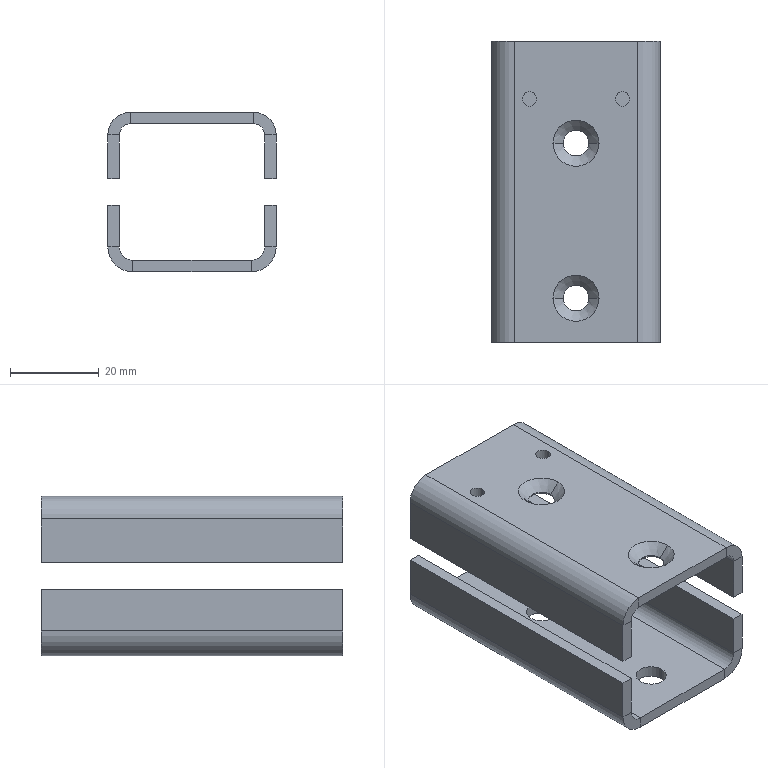Part | STEP file | BASE MICRO | 2 solids | 60 faces | box 38 x 68 x 36 mm | volume 20484 mm3 | plane 36 | cylinder 20 | cone 4 | commonest cylinder face diameters 3.3 x4 5.8 x4 6.8 x4 5 x2 6 x2 10.2 x2
STEP:
#1=CARTESIAN_POINT('',(12.6,45.,-2.3));
#2=VERTEX_POINT('',#1);
#3=CARTESIAN_POINT('',(18.4,45.,-2.3));
#4=VERTEX_POINT('',#3);
#5=CARTESIAN_POINT('',(15.5,45.,-2.3));
#6=DIRECTION('',(0.,0.,1.));
#7=DIRECTION('',(1.,0.,0.));
#8=AXIS2_PLACEMENT_3D('',#5,#6,#7);
#9=CIRCLE('',#8,2.9);
#10=EDGE_CURVE('',#2,#4,#9,.T.);
#11=ORIENTED_EDGE('',*,*,#10,.F.);
#12=CARTESIAN_POINT('',(10.3,45.,0.));
#13=VERTEX_POINT('',#12);
#14=CARTESIAN_POINT('',(10.3,45.,0.));
#15=DIRECTION('',(-0.7071,0.,0.7071));
#16=VECTOR('',#15,1000.);
#17=LINE('',#14,#16);
#18=EDGE_CURVE('',#2,#13,#17,.T.);
#19=ORIENTED_EDGE('',*,*,#18,.T.);
#20=CARTESIAN_POINT('',(20.7,45.,0.));
#21=VERTEX_POINT('',#20);
#22=CARTESIAN_POINT('',(15.5,45.,0.));
#23=DIRECTION('',(0.,0.,1.));
#24=DIRECTION('',(1.,0.,0.));
#25=AXIS2_PLACEMENT_3D('',#22,#23,#24);
#26=CIRCLE('',#25,5.2);
#27=EDGE_CURVE('',#13,#21,#26,.T.);
#28=ORIENTED_EDGE('',*,*,#27,.T.);
#29=CARTESIAN_POINT('',(20.7,45.,0.));
#30=DIRECTION('',(0.7071,0.,0.7071));
#31=VECTOR('',#30,1000.);
#32=LINE('',#29,#31);
#33=EDGE_CURVE('',#4,#21,#32,.T.);
#34=ORIENTED_EDGE('',*,*,#33,.F.);
#35=EDGE_LOOP('',(#11,#19,#28,#34));
#36=FACE_OUTER_BOUND('',#35,.T.);
#37=CARTESIAN_POINT('',(15.5,45.,0.));
#38=DIRECTION('',(0.,0.,1.));
#39=DIRECTION('',(1.,0.,0.));
#40=AXIS2_PLACEMENT_3D('',#37,#38,#39);
#41=CONICAL_SURFACE('',#40,5.2,0.7854);
#42=ADVANCED_FACE('',(#36),#41,.F.);
#43=CARTESIAN_POINT('',(12.6,45.,-2.6));
#44=VERTEX_POINT('',#43);
#45=CARTESIAN_POINT('',(18.4,45.,-2.6));
#46=VERTEX_POINT('',#45);
#47=CARTESIAN_POINT('',(15.5,45.,-2.6));
#48=DIRECTION('',(0.,0.,1.));
#49=DIRECTION('',(1.,0.,0.));
#50=AXIS2_PLACEMENT_3D('',#47,#48,#49);
#51=CIRCLE('',#50,2.9);
#52=EDGE_CURVE('',#44,#46,#51,.T.);
#53=ORIENTED_EDGE('',*,*,#52,.F.);
#54=CARTESIAN_POINT('',(12.6,45.,0.));
#55=DIRECTION('',(0.,0.,1.));
#56=VECTOR('',#55,1000.);
#57=LINE('',#54,#56);
#58=EDGE_CURVE('',#44,#2,#57,.T.);
#59=ORIENTED_EDGE('',*,*,#58,.T.);
#60=ORIENTED_EDGE('',*,*,#10,.T.);
#61=CARTESIAN_POINT('',(18.4,45.,0.));
#62=DIRECTION('',(0.,0.,1.));
#63=VECTOR('',#62,1000.);
#64=LINE('',#61,#63);
#65=EDGE_CURVE('',#46,#4,#64,.T.);
#66=ORIENTED_EDGE('',*,*,#65,.F.);
#67=EDGE_LOOP('',(#53,#59,#60,#66));
#68=FACE_OUTER_BOUND('',#67,.T.);
#69=CARTESIAN_POINT('',(15.5,45.,0.));
#70=DIRECTION('',(0.,0.,1.));
#71=DIRECTION('',(1.,0.,0.));
#72=AXIS2_PLACEMENT_3D('',#69,#70,#71);
#73=CYLINDRICAL_SURFACE('',#72,2.9);
#74=ADVANCED_FACE('',(#68),#73,.F.);
#75=CARTESIAN_POINT('',(12.6,10.,-2.3));
#76=VERTEX_POINT('',#75);
#77=CARTESIAN_POINT('',(18.4,10.,-2.3));
#78=VERTEX_POINT('',#77);
#79=CARTESIAN_POINT('',(15.5,10.,-2.3));
#80=DIRECTION('',(0.,0.,1.));
#81=DIRECTION('',(1.,0.,0.));
#82=AXIS2_PLACEMENT_3D('',#79,#80,#81);
#83=CIRCLE('',#82,2.9);
#84=EDGE_CURVE('',#76,#78,#83,.T.);
#85=ORIENTED_EDGE('',*,*,#84,.F.);
#86=CARTESIAN_POINT('',(10.3,10.,0.));
#87=VERTEX_POINT('',#86);
#88=CARTESIAN_POINT('',(10.3,10.,0.));
#89=DIRECTION('',(-0.7071,0.,0.7071));
#90=VECTOR('',#89,1000.);
#91=LINE('',#88,#90);
#92=EDGE_CURVE('',#76,#87,#91,.T.);
#93=ORIENTED_EDGE('',*,*,#92,.T.);
#94=CARTESIAN_POINT('',(20.7,10.,0.));
#95=VERTEX_POINT('',#94);
#96=CARTESIAN_POINT('',(15.5,10.,0.));
#97=DIRECTION('',(0.,0.,1.));
#98=DIRECTION('',(1.,0.,0.));
#99=AXIS2_PLACEMENT_3D('',#96,#97,#98);
#100=CIRCLE('',#99,5.2);
#101=EDGE_CURVE('',#87,#95,#100,.T.);
#102=ORIENTED_EDGE('',*,*,#101,.T.);
#103=CARTESIAN_POINT('',(20.7,10.,0.));
#104=DIRECTION('',(0.7071,0.,0.7071));
#105=VECTOR('',#104,1000.);
#106=LINE('',#103,#105);
#107=EDGE_CURVE('',#78,#95,#106,.T.);
#108=ORIENTED_EDGE('',*,*,#107,.F.);
#109=EDGE_LOOP('',(#85,#93,#102,#108));
#110=FACE_OUTER_BOUND('',#109,.T.);
#111=CARTESIAN_POINT('',(15.5,10.,0.));
#112=DIRECTION('',(0.,0.,1.));
#113=DIRECTION('',(1.,0.,0.));
#114=AXIS2_PLACEMENT_3D('',#111,#112,#113);
#115=CONICAL_SURFACE('',#114,5.2,0.7854);
#116=ADVANCED_FACE('',(#110),#115,.F.);
#117=CARTESIAN_POINT('',(12.6,10.,-2.6));
#118=VERTEX_POINT('',#117);
#119=CARTESIAN_POINT('',(18.4,10.,-2.6));
#120=VERTEX_POINT('',#119);
#121=CARTESIAN_POINT('',(15.5,10.,-2.6));
#122=DIRECTION('',(0.,0.,1.));
#123=DIRECTION('',(1.,0.,0.));
#124=AXIS2_PLACEMENT_3D('',#121,#122,#123);
#125=CIRCLE('',#124,2.9);
#126=EDGE_CURVE('',#118,#120,#125,.T.);
#127=ORIENTED_EDGE('',*,*,#126,.F.);
#128=CARTESIAN_POINT('',(12.6,10.,0.));
#129=DIRECTION('',(0.,0.,1.));
#130=VECTOR('',#129,1000.);
#131=LINE('',#128,#130);
#132=EDGE_CURVE('',#118,#76,#131,.T.);
#133=ORIENTED_EDGE('',*,*,#132,.T.);
#134=ORIENTED_EDGE('',*,*,#84,.T.);
#135=CARTESIAN_POINT('',(18.4,10.,0.));
#136=DIRECTION('',(0.,0.,1.));
#137=VECTOR('',#136,1000.);
#138=LINE('',#135,#137);
#139=EDGE_CURVE('',#120,#78,#138,.T.);
#140=ORIENTED_EDGE('',*,*,#139,.F.);
#141=EDGE_LOOP('',(#127,#133,#134,#140));
#142=FACE_OUTER_BOUND('',#141,.T.);
#143=CARTESIAN_POINT('',(15.5,10.,0.));
#144=DIRECTION('',(0.,0.,1.));
#145=DIRECTION('',(1.,0.,0.));
#146=AXIS2_PLACEMENT_3D('',#143,#144,#145);
#147=CYLINDRICAL_SURFACE('',#146,2.9);
#148=ADVANCED_FACE('',(#142),#147,.F.);
#149=CARTESIAN_POINT('',(3.35,55.,-2.6));
#150=VERTEX_POINT('',#149);
#151=CARTESIAN_POINT('',(6.65,55.,-2.6));
#152=VERTEX_POINT('',#151);
#153=CARTESIAN_POINT('',(5.,55.,-2.6));
#154=DIRECTION('',(0.,0.,1.));
#155=DIRECTION('',(1.,0.,0.));
#156=AXIS2_PLACEMENT_3D('',#153,#154,#155);
#157=CIRCLE('',#156,1.65);
#158=EDGE_CURVE('',#150,#152,#157,.T.);
#159=ORIENTED_EDGE('',*,*,#158,.F.);
#160=CARTESIAN_POINT('',(3.35,55.,0.));
#161=VERTEX_POINT('',#160);
#162=CARTESIAN_POINT('',(3.35,55.,0.));
#163=DIRECTION('',(0.,0.,1.));
#164=VECTOR('',#163,1000.);
#165=LINE('',#162,#164);
#166=EDGE_CURVE('',#150,#161,#165,.T.);
#167=ORIENTED_EDGE('',*,*,#166,.T.);
#168=CARTESIAN_POINT('',(6.65,55.,0.));
#169=VERTEX_POINT('',#168);
#170=CARTESIAN_POINT('',(5.,55.,0.));
#171=DIRECTION('',(0.,0.,1.));
#172=DIRECTION('',(1.,0.,0.));
#173=AXIS2_PLACEMENT_3D('',#170,#171,#172);
#174=CIRCLE('',#173,1.65);
#175=EDGE_CURVE('',#161,#169,#174,.T.);
#176=ORIENTED_EDGE('',*,*,#175,.T.);
#177=CARTESIAN_POINT('',(6.65,55.,0.));
#178=DIRECTION('',(0.,0.,1.));
#179=VECTOR('',#178,1000.);
#180=LINE('',#177,#179);
#181=EDGE_CURVE('',#152,#169,#180,.T.);
#182=ORIENTED_EDGE('',*,*,#181,.F.);
#183=EDGE_LOOP('',(#159,#167,#176,#182));
#184=FACE_OUTER_BOUND('',#183,.T.);
#185=CARTESIAN_POINT('',(5.,55.,0.));
#186=DIRECTION('',(0.,0.,1.));
#187=DIRECTION('',(1.,0.,0.));
#188=AXIS2_PLACEMENT_3D('',#185,#186,#187);
#189=CYLINDRICAL_SURFACE('',#188,1.65);
#190=ADVANCED_FACE('',(#184),#189,.F.);
#191=CARTESIAN_POINT('',(24.35,55.,-2.6));
#192=VERTEX_POINT('',#191);
#193=CARTESIAN_POINT('',(27.65,55.,-2.6));
#194=VERTEX_POINT('',#193);
#195=CARTESIAN_POINT('',(26.,55.,-2.6));
#196=DIRECTION('',(0.,0.,1.));
#197=DIRECTION('',(1.,0.,0.));
#198=AXIS2_PLACEMENT_3D('',#195,#196,#197);
#199=CIRCLE('',#198,1.65);
#200=EDGE_CURVE('',#192,#194,#199,.T.);
#201=ORIENTED_EDGE('',*,*,#200,.F.);
#202=CARTESIAN_POINT('',(24.35,55.,0.));
#203=VERTEX_POINT('',#202);
#204=CARTESIAN_POINT('',(24.35,55.,0.));
#205=DIRECTION('',(0.,0.,1.));
#206=VECTOR('',#205,1000.);
#207=LINE('',#204,#206);
#208=EDGE_CURVE('',#192,#203,#207,.T.);
#209=ORIENTED_EDGE('',*,*,#208,.T.);
#210=CARTESIAN_POINT('',(27.65,55.,0.));
#211=VERTEX_POINT('',#210);
#212=CARTESIAN_POINT('',(26.,55.,0.));
#213=DIRECTION('',(0.,0.,1.));
#214=DIRECTION('',(1.,0.,0.));
#215=AXIS2_PLACEMENT_3D('',#212,#213,#214);
#216=CIRCLE('',#215,1.65);
#217=EDGE_CURVE('',#203,#211,#216,.T.);
#218=ORIENTED_EDGE('',*,*,#217,.T.);
#219=CARTESIAN_POINT('',(27.65,55.,0.));
#220=DIRECTION('',(0.,0.,1.));
#221=VECTOR('',#220,1000.);
#222=LINE('',#219,#221);
#223=EDGE_CURVE('',#194,#211,#222,.T.);
#224=ORIENTED_EDGE('',*,*,#223,.F.);
#225=EDGE_LOOP('',(#201,#209,#218,#224));
#226=FACE_OUTER_BOUND('',#225,.T.);
#227=CARTESIAN_POINT('',(26.,55.,0.));
#228=DIRECTION('',(0.,0.,1.));
#229=DIRECTION('',(1.,0.,0.));
#230=AXIS2_PLACEMENT_3D('',#227,#228,#229);
#231=CYLINDRICAL_SURFACE('',#230,1.65);
#232=ADVANCED_FACE('',(#226),#231,.F.);
#233=CARTESIAN_POINT('',(29.4,68.,0.));
#234=VERTEX_POINT('',#233);
#235=CARTESIAN_POINT('',(29.4,68.,-2.6));
#236=VERTEX_POINT('',#235);
#237=CARTESIAN_POINT('',(29.4,68.,0.));
#238=DIRECTION('',(0.,0.,-1.));
#239=VECTOR('',#238,1000.);
#240=LINE('',#237,#239);
#241=EDGE_CURVE('',#234,#236,#240,.T.);
#242=ORIENTED_EDGE('',*,*,#241,.F.);
#243=CARTESIAN_POINT('',(34.5,68.,-5.1));
#244=VERTEX_POINT('',#243);
#245=CARTESIAN_POINT('',(29.4,68.,-5.1));
#246=DIRECTION('',(0.,-1.,0.));
#247=DIRECTION('',(0.,0.,1.));
#248=AXIS2_PLACEMENT_3D('',#245,#246,#247);
#249=CIRCLE('',#248,5.1);
#250=EDGE_CURVE('',#244,#234,#249,.T.);
#251=ORIENTED_EDGE('',*,*,#250,.F.);
#252=CARTESIAN_POINT('',(31.9,68.,-5.1));
#253=VERTEX_POINT('',#252);
#254=CARTESIAN_POINT('',(31.9,68.,-5.1));
#255=DIRECTION('',(1.,0.,0.));
#256=VECTOR('',#255,1000.);
#257=LINE('',#254,#256);
#258=EDGE_CURVE('',#253,#244,#257,.T.);
#259=ORIENTED_EDGE('',*,*,#258,.F.);
#260=CARTESIAN_POINT('',(29.4,68.,-5.1));
#261=DIRECTION('',(0.,-1.,0.));
#262=DIRECTION('',(1.,0.,0.));
#263=AXIS2_PLACEMENT_3D('',#260,#261,#262);
#264=CIRCLE('',#263,2.5);
#265=EDGE_CURVE('',#253,#236,#264,.T.);
#266=ORIENTED_EDGE('',*,*,#265,.T.);
#267=EDGE_LOOP('',(#242,#251,#259,#266));
#268=FACE_OUTER_BOUND('',#267,.T.);
#269=CARTESIAN_POINT('',(29.4,68.,0.));
#270=DIRECTION('',(0.,1.,0.));
#271=DIRECTION('',(0.,0.,1.));
#272=AXIS2_PLACEMENT_3D('',#269,#270,#271);
#273=PLANE('',#272);
#274=ADVANCED_FACE('',(#268),#273,.T.);
#275=CARTESIAN_POINT('',(1.6,68.,0.));
#276=VERTEX_POINT('',#275);
#277=CARTESIAN_POINT('',(-3.5,68.,0.));
#278=DIRECTION('',(-1.,0.,0.));
#279=VECTOR('',#278,1000.);
#280=LINE('',#277,#279);
#281=EDGE_CURVE('',#234,#276,#280,.T.);
#282=ORIENTED_EDGE('',*,*,#281,.F.);
#283=ORIENTED_EDGE('',*,*,#241,.T.);
#284=CARTESIAN_POINT('',(1.6,68.,-2.6));
#285=VERTEX_POINT('',#284);
#286=CARTESIAN_POINT('',(-3.5,68.,-2.6));
#287=DIRECTION('',(-1.,0.,0.));
#288=VECTOR('',#287,1000.);
#289=LINE('',#286,#288);
#290=EDGE_CURVE('',#236,#285,#289,.T.);
#291=ORIENTED_EDGE('',*,*,#290,.T.);
#292=CARTESIAN_POINT('',(1.6,68.,-2.6));
#293=DIRECTION('',(0.,0.,1.));
#294=VECTOR('',#293,1000.);
#295=LINE('',#292,#294);
#296=EDGE_CURVE('',#285,#276,#295,.T.);
#297=ORIENTED_EDGE('',*,*,#296,.T.);
#298=EDGE_LOOP('',(#282,#283,#291,#297));
#299=FACE_OUTER_BOUND('',#298,.T.);
#300=CARTESIAN_POINT('',(31.9,68.,-5.1));
#301=DIRECTION('',(0.,1.,0.));
#302=DIRECTION('',(0.,0.,1.));
#303=AXIS2_PLACEMENT_3D('',#300,#301,#302);
#304=PLANE('',#303);
#305=ADVANCED_FACE('',(#299),#304,.T.);
#306=CARTESIAN_POINT('',(34.5,0.,-5.1));
#307=VERTEX_POINT('',#306);
#308=CARTESIAN_POINT('',(31.9,0.,-5.1));
#309=VERTEX_POINT('',#308);
#310=CARTESIAN_POINT('',(34.5,0.,-5.1));
#311=DIRECTION('',(-1.,0.,0.));
#312=VECTOR('',#311,1000.);
#313=LINE('',#310,#312);
#314=EDGE_CURVE('',#307,#309,#313,.T.);
#315=ORIENTED_EDGE('',*,*,#314,.F.);
#316=CARTESIAN_POINT('',(29.4,0.,0.));
#317=VERTEX_POINT('',#316);
#318=CARTESIAN_POINT('',(29.4,0.,-5.1));
#319=DIRECTION('',(0.,-1.,0.));
#320=DIRECTION('',(0.,0.,1.));
#321=AXIS2_PLACEMENT_3D('',#318,#319,#320);
#322=CIRCLE('',#321,5.1);
#323=EDGE_CURVE('',#307,#317,#322,.T.);
#324=ORIENTED_EDGE('',*,*,#323,.T.);
#325=CARTESIAN_POINT('',(29.4,0.,-2.6));
#326=VERTEX_POINT('',#325);
#327=CARTESIAN_POINT('',(29.4,0.,-2.6));
#328=DIRECTION('',(0.,0.,1.));
#329=VECTOR('',#328,1000.);
#330=LINE('',#327,#329);
#331=EDGE_CURVE('',#326,#317,#330,.T.);
#332=ORIENTED_EDGE('',*,*,#331,.F.);
#333=CARTESIAN_POINT('',(29.4,0.,-5.1));
#334=DIRECTION('',(0.,-1.,0.));
#335=DIRECTION('',(1.,0.,0.));
#336=AXIS2_PLACEMENT_3D('',#333,#334,#335);
#337=CIRCLE('',#336,2.5);
#338=EDGE_CURVE('',#309,#326,#337,.T.);
#339=ORIENTED_EDGE('',*,*,#338,.F.);
#340=EDGE_LOOP('',(#315,#324,#332,#339));
#341=FACE_OUTER_BOUND('',#340,.T.);
#342=CARTESIAN_POINT('',(34.5,0.,-5.1));
#343=DIRECTION('',(0.,-1.,0.));
#344=DIRECTION('',(0.,0.,-1.));
#345=AXIS2_PLACEMENT_3D('',#342,#343,#344);
#346=PLANE('',#345);
#347=ADVANCED_FACE('',(#341),#346,.T.);
#348=CARTESIAN_POINT('',(34.5,0.,-15.));
#349=VERTEX_POINT('',#348);
#350=CARTESIAN_POINT('',(34.5,0.,0.));
#351=DIRECTION('',(0.,0.,1.));
#352=VECTOR('',#351,1000.);
#353=LINE('',#350,#352);
#354=EDGE_CURVE('',#349,#307,#353,.T.);
#355=ORIENTED_EDGE('',*,*,#354,.T.);
#356=ORIENTED_EDGE('',*,*,#314,.T.);
#357=CARTESIAN_POINT('',(31.9,0.,-15.));
#358=VERTEX_POINT('',#357);
#359=CARTESIAN_POINT('',(31.9,0.,0.));
#360=DIRECTION('',(0.,0.,1.));
#361=VECTOR('',#360,1000.);
#362=LINE('',#359,#361);
#363=EDGE_CURVE('',#358,#309,#362,.T.);
#364=ORIENTED_EDGE('',*,*,#363,.F.);
#365=CARTESIAN_POINT('',(31.9,0.,-15.));
#366=DIRECTION('',(1.,0.,0.));
#367=VECTOR('',#366,1000.);
#368=LINE('',#365,#367);
#369=EDGE_CURVE('',#358,#349,#368,.T.);
#370=ORIENTED_EDGE('',*,*,#369,.T.);
#371=EDGE_LOOP('',(#355,#356,#364,#370));
#372=FACE_OUTER_BOUND('',#371,.T.);
#373=CARTESIAN_POINT('',(29.4,0.,-2.6));
#374=DIRECTION('',(0.,-1.,0.));
#375=DIRECTION('',(0.,0.,-1.));
#376=AXIS2_PLACEMENT_3D('',#373,#374,#375);
#377=PLANE('',#376);
#378=ADVANCED_FACE('',(#372),#377,.T.);
#379=CARTESIAN_POINT('',(-3.5,68.,-5.1));
#380=VERTEX_POINT('',#379);
#381=CARTESIAN_POINT('',(-0.9,68.,-5.1));
#382=VERTEX_POINT('',#381);
#383=CARTESIAN_POINT('',(-3.5,68.,-5.1));
#384=DIRECTION('',(1.,0.,0.));
#385=VECTOR('',#384,1000.);
#386=LINE('',#383,#385);
#387=EDGE_CURVE('',#380,#382,#386,.T.);
#388=ORIENTED_EDGE('',*,*,#387,.F.);
#389=CARTESIAN_POINT('',(1.6,68.,-5.1));
#390=DIRECTION('',(0.,-1.,0.));
#391=DIRECTION('',(0.,0.,1.));
#392=AXIS2_PLACEMENT_3D('',#389,#390,#391);
#393=CIRCLE('',#392,5.1);
#394=EDGE_CURVE('',#276,#380,#393,.T.);
#395=ORIENTED_EDGE('',*,*,#394,.F.);
#396=ORIENTED_EDGE('',*,*,#296,.F.);
#397=CARTESIAN_POINT('',(1.6,68.,-5.1));
#398=DIRECTION('',(0.,-1.,0.));
#399=DIRECTION('',(1.,0.,0.));
#400=AXIS2_PLACEMENT_3D('',#397,#398,#399);
#401=CIRCLE('',#400,2.5);
#402=EDGE_CURVE('',#285,#382,#401,.T.);
#403=ORIENTED_EDGE('',*,*,#402,.T.);
#404=EDGE_LOOP('',(#388,#395,#396,#403));
#405=FACE_OUTER_BOUND('',#404,.T.);
#406=CARTESIAN_POINT('',(-3.5,68.,-5.1));
#407=DIRECTION('',(0.,1.,0.));
#408=DIRECTION('',(0.,0.,1.));
#409=AXIS2_PLACEMENT_3D('',#406,#407,#408);
#410=PLANE('',#409);
#411=ADVANCED_FACE('',(#405),#410,.T.);
#412=CARTESIAN_POINT('',(-3.5,68.,-15.));
#413=VERTEX_POINT('',#412);
#414=CARTESIAN_POINT('',(-3.5,68.,0.));
#415=DIRECTION('',(0.,0.,-1.));
#416=VECTOR('',#415,1000.);
#417=LINE('',#414,#416);
#418=EDGE_CURVE('',#380,#413,#417,.T.);
#419=ORIENTED_EDGE('',*,*,#418,.F.);
#420=ORIENTED_EDGE('',*,*,#387,.T.);
#421=CARTESIAN_POINT('',(-0.9,68.,-15.));
#422=VERTEX_POINT('',#421);
#423=CARTESIAN_POINT('',(-0.9,68.,0.));
#424=DIRECTION('',(0.,0.,-1.));
#425=VECTOR('',#424,1000.);
#426=LINE('',#423,#425);
#427=EDGE_CURVE('',#382,#422,#426,.T.);
#428=ORIENTED_EDGE('',*,*,#427,.T.);
#429=CARTESIAN_POINT('',(-3.5,68.,-15.));
#430=DIRECTION('',(1.,0.,0.));
#431=VECTOR('',#430,1000.);
#432=LINE('',#429,#431);
#433=EDGE_CURVE('',#413,#422,#432,.T.);
#434=ORIENTED_EDGE('',*,*,#433,.F.);
#435=EDGE_LOOP('',(#419,#420,#428,#434));
#436=FACE_OUTER_BOUND('',#435,.T.);
#437=CARTESIAN_POINT('',(1.6,68.,-2.6));
#438=DIRECTION('',(0.,1.,0.));
#439=DIRECTION('',(0.,0.,1.));
#440=AXIS2_PLACEMENT_3D('',#437,#438,#439);
#441=PLANE('',#440);
#442=ADVANCED_FACE('',(#436),#441,.T.);
#443=CARTESIAN_POINT('',(1.6,0.,0.));
#444=VERTEX_POINT('',#443);
#445=CARTESIAN_POINT('',(1.6,0.,-2.6));
#446=VERTEX_POINT('',#445);
#447=CARTESIAN_POINT('',(1.6,0.,0.));
#448=DIRECTION('',(0.,0.,-1.));
#449=VECTOR('',#448,1000.);
#450=LINE('',#447,#449);
#451=EDGE_CURVE('',#444,#446,#450,.T.);
#452=ORIENTED_EDGE('',*,*,#451,.F.);
#453=CARTESIAN_POINT('',(-3.5,0.,-5.1));
#454=VERTEX_POINT('',#453);
#455=CARTESIAN_POINT('',(1.6,0.,-5.1));
#456=DIRECTION('',(0.,-1.,0.));
#457=DIRECTION('',(0.,0.,1.));
#458=AXIS2_PLACEMENT_3D('',#455,#456,#457);
#459=CIRCLE('',#458,5.1);
#460=EDGE_CURVE('',#444,#454,#459,.T.);
#461=ORIENTED_EDGE('',*,*,#460,.T.);
#462=CARTESIAN_POINT('',(-0.9,0.,-5.1));
#463=VERTEX_POINT('',#462);
#464=CARTESIAN_POINT('',(-0.9,0.,-5.1));
#465=DIRECTION('',(-1.,0.,0.));
#466=VECTOR('',#465,1000.);
#467=LINE('',#464,#466);
#468=EDGE_CURVE('',#463,#454,#467,.T.);
#469=ORIENTED_EDGE('',*,*,#468,.F.);
#470=CARTESIAN_POINT('',(1.6,0.,-5.1));
#471=DIRECTION('',(0.,-1.,0.));
#472=DIRECTION('',(1.,0.,0.));
#473=AXIS2_PLACEMENT_3D('',#470,#471,#472);
#474=CIRCLE('',#473,2.5);
#475=EDGE_CURVE('',#446,#463,#474,.T.);
#476=ORIENTED_EDGE('',*,*,#475,.F.);
#477=EDGE_LOOP('',(#452,#461,#469,#476));
#478=FACE_OUTER_BOUND('',#477,.T.);
#479=CARTESIAN_POINT('',(1.6,0.,0.));
#480=DIRECTION('',(0.,-1.,0.));
#481=DIRECTION('',(0.,0.,-1.));
#482=AXIS2_PLACEMENT_3D('',#479,#480,#481);
#483=PLANE('',#482);
#484=ADVANCED_FACE('',(#478),#483,.T.);
#485=CARTESIAN_POINT('',(-3.5,0.,0.));
#486=DIRECTION('',(-1.,0.,0.));
#487=VECTOR('',#486,1000.);
#488=LINE('',#485,#487);
#489=EDGE_CURVE('',#317,#444,#488,.T.);
#490=ORIENTED_EDGE('',*,*,#489,.T.);
#491=ORIENTED_EDGE('',*,*,#451,.T.);
#492=CARTESIAN_POINT('',(-3.5,0.,-2.6));
#493=DIRECTION('',(-1.,0.,0.));
#494=VECTOR('',#493,1000.);
#495=LINE('',#492,#494);
#496=EDGE_CURVE('',#326,#446,#495,.T.);
#497=ORIENTED_EDGE('',*,*,#496,.F.);
#498=ORIENTED_EDGE('',*,*,#331,.T.);
#499=EDGE_LOOP('',(#490,#491,#497,#498));
#500=FACE_OUTER_BOUND('',#499,.T.);
#501=CARTESIAN_POINT('',(-0.9,0.,-5.1));
#502=DIRECTION('',(0.,-1.,0.));
#503=DIRECTION('',(0.,0.,-1.));
#504=AXIS2_PLACEMENT_3D('',#501,#502,#503);
#505=PLANE('',#504);
#506=ADVANCED_FACE('',(#500),#505,.T.);
#507=CARTESIAN_POINT('',(-0.9,0.,-15.));
#508=VERTEX_POINT('',#507);
#509=CARTESIAN_POINT('',(-0.9,0.,0.));
#510=DIRECTION('',(0.,0.,-1.));
#511=VECTOR('',#510,1000.);
#512=LINE('',#509,#511);
#513=EDGE_CURVE('',#463,#508,#512,.T.);
#514=ORIENTED_EDGE('',*,*,#513,.T.);
#515=CARTESIAN_POINT('',(-0.9,68.,-15.));
#516=DIRECTION('',(0.,-1.,0.));
#517=VECTOR('',#516,1000.);
#518=LINE('',#515,#517);
#519=EDGE_CURVE('',#422,#508,#518,.T.);
#520=ORIENTED_EDGE('',*,*,#519,.F.);
#521=ORIENTED_EDGE('',*,*,#427,.F.);
#522=CARTESIAN_POINT('',(-0.9,68.,-5.1));
#523=DIRECTION('',(0.,-1.,0.));
#524=VECTOR('',#523,1000.);
#525=LINE('',#522,#524);
#526=EDGE_CURVE('',#382,#463,#525,.T.);
#527=ORIENTED_EDGE('',*,*,#526,.T.);
#528=EDGE_LOOP('',(#514,#520,#521,#527));
#529=FACE_OUTER_BOUND('',#528,.T.);
#530=CARTESIAN_POINT('',(-0.9,68.,0.));
#531=DIRECTION('',(-1.,0.,0.));
#532=DIRECTION('',(0.,0.,1.));
#533=AXIS2_PLACEMENT_3D('',#530,#531,#532);
#534=PLANE('',#533);
#535=ADVANCED_FACE('',(#529),#534,.F.);
#536=CARTESIAN_POINT('',(-3.5,0.,-15.));
#537=VERTEX_POINT('',#536);
#538=CARTESIAN_POINT('',(-3.5,0.,-15.));
#539=DIRECTION('',(1.,0.,0.));
#540=VECTOR('',#539,1000.);
#541=LINE('',#538,#540);
#542=EDGE_CURVE('',#537,#508,#541,.T.);
#543=ORIENTED_EDGE('',*,*,#542,.F.);
#544=CARTESIAN_POINT('',(-3.5,68.,-15.));
#545=DIRECTION('',(0.,-1.,0.));
#546=VECTOR('',#545,1000.);
#547=LINE('',#544,#546);
#548=EDGE_CURVE('',#413,#537,#547,.T.);
#549=ORIENTED_EDGE('',*,*,#548,.F.);
#550=ORIENTED_EDGE('',*,*,#433,.T.);
#551=ORIENTED_EDGE('',*,*,#519,.T.);
#552=EDGE_LOOP('',(#543,#549,#550,#551));
#553=FACE_OUTER_BOUND('',#552,.T.);
#554=CARTESIAN_POINT('',(-3.5,68.,-15.));
#555=DIRECTION('',(0.,0.,-1.));
#556=DIRECTION('',(-1.,0.,0.));
#557=AXIS2_PLACEMENT_3D('',#554,#555,#556);
#558=PLANE('',#557);
#559=ADVANCED_FACE('',(#553),#558,.T.);
#560=CARTESIAN_POINT('',(-3.5,0.,0.));
#561=DIRECTION('',(0.,0.,-1.));
#562=VECTOR('',#561,1000.);
#563=LINE('',#560,#562);
#564=EDGE_CURVE('',#454,#537,#563,.T.);
#565=ORIENTED_EDGE('',*,*,#564,.F.);
#566=CARTESIAN_POINT('',(-3.5,68.,-5.1));
#567=DIRECTION('',(0.,-1.,0.));
#568=VECTOR('',#567,1000.);
#569=LINE('',#566,#568);
#570=EDGE_CURVE('',#380,#454,#569,.T.);
#571=ORIENTED_EDGE('',*,*,#570,.F.);
#572=ORIENTED_EDGE('',*,*,#418,.T.);
#573=ORIENTED_EDGE('',*,*,#548,.T.);
#574=EDGE_LOOP('',(#565,#571,#572,#573));
#575=FACE_OUTER_BOUND('',#574,.T.);
#576=CARTESIAN_POINT('',(-3.5,68.,0.));
#577=DIRECTION('',(-1.,0.,0.));
#578=DIRECTION('',(0.,0.,1.));
#579=AXIS2_PLACEMENT_3D('',#576,#577,#578);
#580=PLANE('',#579);
#581=ADVANCED_FACE('',(#575),#580,.T.);
#582=ORIENTED_EDGE('',*,*,#460,.F.);
#583=CARTESIAN_POINT('',(1.6,68.,0.));
#584=DIRECTION('',(0.,-1.,0.));
#585=VECTOR('',#584,1000.);
#586=LINE('',#583,#585);
#587=EDGE_CURVE('',#276,#444,#586,.T.);
#588=ORIENTED_EDGE('',*,*,#587,.F.);
#589=ORIENTED_EDGE('',*,*,#394,.T.);
#590=ORIENTED_EDGE('',*,*,#570,.T.);
#591=EDGE_LOOP('',(#582,#588,#589,#590));
#592=FACE_OUTER_BOUND('',#591,.T.);
#593=CARTESIAN_POINT('',(1.6,68.,-5.1));
#594=DIRECTION('',(0.,-1.,0.));
#595=DIRECTION('',(0.,0.,-1.));
#596=AXIS2_PLACEMENT_3D('',#593,#594,#595);
#597=CYLINDRICAL_SURFACE('',#596,5.1);
#598=ADVANCED_FACE('',(#592),#597,.T.);
#599=CARTESIAN_POINT('',(15.5,45.,0.));
#600=DIRECTION('',(0.,0.,1.));
#601=DIRECTION('',(1.,0.,0.));
#602=AXIS2_PLACEMENT_3D('',#599,#600,#601);
#603=CIRCLE('',#602,5.2);
#604=EDGE_CURVE('',#21,#13,#603,.T.);
#605=ORIENTED_EDGE('',*,*,#604,.F.);
#606=ORIENTED_EDGE('',*,*,#27,.F.);
#607=EDGE_LOOP('',(#605,#606));
#608=FACE_BOUND('',#607,.T.);
#609=CARTESIAN_POINT('',(15.5,10.,0.));
#610=DIRECTION('',(0.,0.,1.));
#611=DIRECTION('',(1.,0.,0.));
#612=AXIS2_PLACEMENT_3D('',#609,#610,#611);
#613=CIRCLE('',#612,5.2);
#614=EDGE_CURVE('',#95,#87,#613,.T.);
#615=ORIENTED_EDGE('',*,*,#614,.F.);
#616=ORIENTED_EDGE('',*,*,#101,.F.);
#617=EDGE_LOOP('',(#615,#616));
#618=FACE_BOUND('',#617,.T.);
#619=CARTESIAN_POINT('',(5.,55.,0.));
#620=DIRECTION('',(0.,0.,1.));
#621=DIRECTION('',(1.,0.,0.));
#622=AXIS2_PLACEMENT_3D('',#619,#620,#621);
#623=CIRCLE('',#622,1.65);
#624=EDGE_CURVE('',#169,#161,#623,.T.);
#625=ORIENTED_EDGE('',*,*,#624,.F.);
#626=ORIENTED_EDGE('',*,*,#175,.F.);
#627=EDGE_LOOP('',(#625,#626));
#628=FACE_BOUND('',#627,.T.);
#629=CARTESIAN_POINT('',(26.,55.,0.));
#630=DIRECTION('',(0.,0.,1.));
#631=DIRECTION('',(1.,0.,0.));
#632=AXIS2_PLACEMENT_3D('',#629,#630,#631);
#633=CIRCLE('',#632,1.65);
#634=EDGE_CURVE('',#211,#203,#633,.T.);
#635=ORIENTED_EDGE('',*,*,#634,.F.);
#636=ORIENTED_EDGE('',*,*,#217,.F.);
#637=EDGE_LOOP('',(#635,#636));
#638=FACE_BOUND('',#637,.T.);
#639=ORIENTED_EDGE('',*,*,#489,.F.);
#640=CARTESIAN_POINT('',(29.4,68.,0.));
#641=DIRECTION('',(0.,-1.,0.));
#642=VECTOR('',#641,1000.);
#643=LINE('',#640,#642);
#644=EDGE_CURVE('',#234,#317,#643,.T.);
#645=ORIENTED_EDGE('',*,*,#644,.F.);
#646=ORIENTED_EDGE('',*,*,#281,.T.);
#647=ORIENTED_EDGE('',*,*,#587,.T.);
#648=EDGE_LOOP('',(#639,#645,#646,#647));
#649=FACE_OUTER_BOUND('',#648,.T.);
#650=CARTESIAN_POINT('',(-3.5,68.,0.));
#651=DIRECTION('',(0.,0.,1.));
#652=DIRECTION('',(1.,0.,0.));
#653=AXIS2_PLACEMENT_3D('',#650,#651,#652);
#654=PLANE('',#653);
#655=ADVANCED_FACE('',(#608,#618,#628,#638,#649),#654,.T.);
#656=ORIENTED_EDGE('',*,*,#323,.F.);
#657=CARTESIAN_POINT('',(34.5,68.,-5.1));
#658=DIRECTION('',(0.,-1.,0.));
#659=VECTOR('',#658,1000.);
#660=LINE('',#657,#659);
#661=EDGE_CURVE('',#244,#307,#660,.T.);
#662=ORIENTED_EDGE('',*,*,#661,.F.);
#663=ORIENTED_EDGE('',*,*,#250,.T.);
#664=ORIENTED_EDGE('',*,*,#644,.T.);
#665=EDGE_LOOP('',(#656,#662,#663,#664));
#666=FACE_OUTER_BOUND('',#665,.T.);
#667=CARTESIAN_POINT('',(29.4,68.,-5.1));
#668=DIRECTION('',(0.,-1.,0.));
#669=DIRECTION('',(0.,0.,-1.));
#670=AXIS2_PLACEMENT_3D('',#667,#668,#669);
#671=CYLINDRICAL_SURFACE('',#670,5.1);
#672=ADVANCED_FACE('',(#666),#671,.T.);
#673=ORIENTED_EDGE('',*,*,#354,.F.);
#674=CARTESIAN_POINT('',(34.5,68.,-15.));
#675=VERTEX_POINT('',#674);
#676=CARTESIAN_POINT('',(34.5,68.,-15.));
#677=DIRECTION('',(0.,-1.,0.));
#678=VECTOR('',#677,1000.);
#679=LINE('',#676,#678);
#680=EDGE_CURVE('',#675,#349,#679,.T.);
#681=ORIENTED_EDGE('',*,*,#680,.F.);
#682=CARTESIAN_POINT('',(34.5,68.,0.));
#683=DIRECTION('',(0.,0.,1.));
#684=VECTOR('',#683,1000.);
#685=LINE('',#682,#684);
#686=EDGE_CURVE('',#675,#244,#685,.T.);
#687=ORIENTED_EDGE('',*,*,#686,.T.);
#688=ORIENTED_EDGE('',*,*,#661,.T.);
#689=EDGE_LOOP('',(#673,#681,#687,#688));
#690=FACE_OUTER_BOUND('',#689,.T.);
#691=CARTESIAN_POINT('',(34.5,68.,0.));
#692=DIRECTION('',(1.,0.,0.));
#693=DIRECTION('',(0.,0.,-1.));
#694=AXIS2_PLACEMENT_3D('',#691,#692,#693);
#695=PLANE('',#694);
#696=ADVANCED_FACE('',(#690),#695,.T.);
#697=ORIENTED_EDGE('',*,*,#369,.F.);
#698=CARTESIAN_POINT('',(31.9,68.,-15.));
#699=VERTEX_POINT('',#698);
#700=CARTESIAN_POINT('',(31.9,68.,-15.));
#701=DIRECTION('',(0.,-1.,0.));
#702=VECTOR('',#701,1000.);
#703=LINE('',#700,#702);
#704=EDGE_CURVE('',#699,#358,#703,.T.);
#705=ORIENTED_EDGE('',*,*,#704,.F.);
#706=CARTESIAN_POINT('',(31.9,68.,-15.));
#707=DIRECTION('',(1.,0.,0.));
#708=VECTOR('',#707,1000.);
#709=LINE('',#706,#708);
#710=EDGE_CURVE('',#699,#675,#709,.T.);
#711=ORIENTED_EDGE('',*,*,#710,.T.);
#712=ORIENTED_EDGE('',*,*,#680,.T.);
#713=EDGE_LOOP('',(#697,#705,#711,#712));
#714=FACE_OUTER_BOUND('',#713,.T.);
#715=CARTESIAN_POINT('',(31.9,68.,-15.));
#716=DIRECTION('',(0.,0.,-1.));
#717=DIRECTION('',(-1.,0.,0.));
#718=AXIS2_PLACEMENT_3D('',#715,#716,#717);
#719=PLANE('',#718);
#720=ADVANCED_FACE('',(#714),#719,.T.);
#721=ORIENTED_EDGE('',*,*,#363,.T.);
#722=CARTESIAN_POINT('',(31.9,68.,-5.1));
#723=DIRECTION('',(0.,-1.,0.));
#724=VECTOR('',#723,1000.);
#725=LINE('',#722,#724);
#726=EDGE_CURVE('',#253,#309,#725,.T.);
#727=ORIENTED_EDGE('',*,*,#726,.F.);
#728=CARTESIAN_POINT('',(31.9,68.,0.));
#729=DIRECTION('',(0.,0.,1.));
#730=VECTOR('',#729,1000.);
#731=LINE('',#728,#730);
#732=EDGE_CURVE('',#699,#253,#731,.T.);
#733=ORIENTED_EDGE('',*,*,#732,.F.);
#734=ORIENTED_EDGE('',*,*,#704,.T.);
#735=EDGE_LOOP('',(#721,#727,#733,#734));
#736=FACE_OUTER_BOUND('',#735,.T.);
#737=CARTESIAN_POINT('',(31.9,68.,0.));
#738=DIRECTION('',(1.,0.,0.));
#739=DIRECTION('',(0.,0.,-1.));
#740=AXIS2_PLACEMENT_3D('',#737,#738,#739);
#741=PLANE('',#740);
#742=ADVANCED_FACE('',(#736),#741,.F.);
#743=ORIENTED_EDGE('',*,*,#338,.T.);
#744=CARTESIAN_POINT('',(29.4,68.,-2.6));
#745=DIRECTION('',(0.,-1.,0.));
#746=VECTOR('',#745,1000.);
#747=LINE('',#744,#746);
#748=EDGE_CURVE('',#236,#326,#747,.T.);
#749=ORIENTED_EDGE('',*,*,#748,.F.);
#750=ORIENTED_EDGE('',*,*,#265,.F.);
#751=ORIENTED_EDGE('',*,*,#726,.T.);
#752=EDGE_LOOP('',(#743,#749,#750,#751));
#753=FACE_OUTER_BOUND('',#752,.T.);
#754=CARTESIAN_POINT('',(29.4,68.,-5.1));
#755=DIRECTION('',(0.,-1.,0.));
#756=DIRECTION('',(0.,0.,-1.));
#757=AXIS2_PLACEMENT_3D('',#754,#755,#756);
#758=CYLINDRICAL_SURFACE('',#757,2.5);
#759=ADVANCED_FACE('',(#753),#758,.F.);
#760=CARTESIAN_POINT('',(15.5,45.,-2.6));
#761=DIRECTION('',(0.,0.,1.));
#762=DIRECTION('',(1.,0.,0.));
#763=AXIS2_PLACEMENT_3D('',#760,#761,#762);
#764=CIRCLE('',#763,2.9);
#765=EDGE_CURVE('',#46,#44,#764,.T.);
#766=ORIENTED_EDGE('',*,*,#765,.T.);
#767=ORIENTED_EDGE('',*,*,#52,.T.);
#768=EDGE_LOOP('',(#766,#767));
#769=FACE_BOUND('',#768,.T.);
#770=CARTESIAN_POINT('',(15.5,10.,-2.6));
#771=DIRECTION('',(0.,0.,1.));
#772=DIRECTION('',(1.,0.,0.));
#773=AXIS2_PLACEMENT_3D('',#770,#771,#772);
#774=CIRCLE('',#773,2.9);
#775=EDGE_CURVE('',#120,#118,#774,.T.);
#776=ORIENTED_EDGE('',*,*,#775,.T.);
#777=ORIENTED_EDGE('',*,*,#126,.T.);
#778=EDGE_LOOP('',(#776,#777));
#779=FACE_BOUND('',#778,.T.);
#780=CARTESIAN_POINT('',(5.,55.,-2.6));
#781=DIRECTION('',(0.,0.,1.));
#782=DIRECTION('',(1.,0.,0.));
#783=AXIS2_PLACEMENT_3D('',#780,#781,#782);
#784=CIRCLE('',#783,1.65);
#785=EDGE_CURVE('',#152,#150,#784,.T.);
#786=ORIENTED_EDGE('',*,*,#785,.T.);
#787=ORIENTED_EDGE('',*,*,#158,.T.);
#788=EDGE_LOOP('',(#786,#787));
#789=FACE_BOUND('',#788,.T.);
#790=CARTESIAN_POINT('',(26.,55.,-2.6));
#791=DIRECTION('',(0.,0.,1.));
#792=DIRECTION('',(1.,0.,0.));
#793=AXIS2_PLACEMENT_3D('',#790,#791,#792);
#794=CIRCLE('',#793,1.65);
#795=EDGE_CURVE('',#194,#192,#794,.T.);
#796=ORIENTED_EDGE('',*,*,#795,.T.);
#797=ORIENTED_EDGE('',*,*,#200,.T.);
#798=EDGE_LOOP('',(#796,#797));
#799=FACE_BOUND('',#798,.T.);
#800=ORIENTED_EDGE('',*,*,#496,.T.);
#801=CARTESIAN_POINT('',(1.6,68.,-2.6));
#802=DIRECTION('',(0.,-1.,0.));
#803=VECTOR('',#802,1000.);
#804=LINE('',#801,#803);
#805=EDGE_CURVE('',#285,#446,#804,.T.);
#806=ORIENTED_EDGE('',*,*,#805,.F.);
#807=ORIENTED_EDGE('',*,*,#290,.F.);
#808=ORIENTED_EDGE('',*,*,#748,.T.);
#809=EDGE_LOOP('',(#800,#806,#807,#808));
#810=FACE_OUTER_BOUND('',#809,.T.);
#811=CARTESIAN_POINT('',(-3.5,68.,-2.6));
#812=DIRECTION('',(0.,0.,1.));
#813=DIRECTION('',(1.,0.,0.));
#814=AXIS2_PLACEMENT_3D('',#811,#812,#813);
#815=PLANE('',#814);
#816=ADVANCED_FACE('',(#769,#779,#789,#799,#810),#815,.F.);
#817=ORIENTED_EDGE('',*,*,#475,.T.);
#818=ORIENTED_EDGE('',*,*,#526,.F.);
#819=ORIENTED_EDGE('',*,*,#402,.F.);
#820=ORIENTED_EDGE('',*,*,#805,.T.);
#821=EDGE_LOOP('',(#817,#818,#819,#820));
#822=FACE_OUTER_BOUND('',#821,.T.);
#823=CARTESIAN_POINT('',(1.6,68.,-5.1));
#824=DIRECTION('',(0.,-1.,0.));
#825=DIRECTION('',(0.,0.,-1.));
#826=AXIS2_PLACEMENT_3D('',#823,#824,#825);
#827=CYLINDRICAL_SURFACE('',#826,2.5);
#828=ADVANCED_FACE('',(#822),#827,.F.);
#829=ORIENTED_EDGE('',*,*,#732,.T.);
#830=ORIENTED_EDGE('',*,*,#258,.T.);
#831=ORIENTED_EDGE('',*,*,#686,.F.);
#832=ORIENTED_EDGE('',*,*,#710,.F.);
#833=EDGE_LOOP('',(#829,#830,#831,#832));
#834=FACE_OUTER_BOUND('',#833,.T.);
#835=CARTESIAN_POINT('',(1.6,68.,-5.1));
#836=DIRECTION('',(0.,1.,0.));
#837=DIRECTION('',(1.,0.,0.));
#838=AXIS2_PLACEMENT_3D('',#835,#836,#837);
#839=PLANE('',#838);
#840=ADVANCED_FACE('',(#834),#839,.T.);
#841=ORIENTED_EDGE('',*,*,#513,.F.);
#842=ORIENTED_EDGE('',*,*,#468,.T.);
#843=ORIENTED_EDGE('',*,*,#564,.T.);
#844=ORIENTED_EDGE('',*,*,#542,.T.);
#845=EDGE_LOOP('',(#841,#842,#843,#844));
#846=FACE_OUTER_BOUND('',#845,.T.);
#847=CARTESIAN_POINT('',(1.6,0.,-5.1));
#848=DIRECTION('',(0.,1.,0.));
#849=DIRECTION('',(1.,0.,0.));
#850=AXIS2_PLACEMENT_3D('',#847,#848,#849);
#851=PLANE('',#850);
#852=ADVANCED_FACE('',(#846),#851,.F.);
#853=ORIENTED_EDGE('',*,*,#208,.F.);
#854=ORIENTED_EDGE('',*,*,#795,.F.);
#855=ORIENTED_EDGE('',*,*,#223,.T.);
#856=ORIENTED_EDGE('',*,*,#634,.T.);
#857=EDGE_LOOP('',(#853,#854,#855,#856));
#858=FACE_OUTER_BOUND('',#857,.T.);
#859=CARTESIAN_POINT('',(26.,55.,0.));
#860=DIRECTION('',(0.,0.,1.));
#861=DIRECTION('',(1.,0.,0.));
#862=AXIS2_PLACEMENT_3D('',#859,#860,#861);
#863=CYLINDRICAL_SURFACE('',#862,1.65);
#864=ADVANCED_FACE('',(#858),#863,.F.);
#865=ORIENTED_EDGE('',*,*,#166,.F.);
#866=ORIENTED_EDGE('',*,*,#785,.F.);
#867=ORIENTED_EDGE('',*,*,#181,.T.);
#868=ORIENTED_EDGE('',*,*,#624,.T.);
#869=EDGE_LOOP('',(#865,#866,#867,#868));
#870=FACE_OUTER_BOUND('',#869,.T.);
#871=CARTESIAN_POINT('',(5.,55.,0.));
#872=DIRECTION('',(0.,0.,1.));
#873=DIRECTION('',(1.,0.,0.));
#874=AXIS2_PLACEMENT_3D('',#871,#872,#873);
#875=CYLINDRICAL_SURFACE('',#874,1.65);
#876=ADVANCED_FACE('',(#870),#875,.F.);
#877=ORIENTED_EDGE('',*,*,#132,.F.);
#878=ORIENTED_EDGE('',*,*,#775,.F.);
#879=ORIENTED_EDGE('',*,*,#139,.T.);
#880=CARTESIAN_POINT('',(15.5,10.,-2.3));
#881=DIRECTION('',(0.,0.,1.));
#882=DIRECTION('',(1.,0.,0.));
#883=AXIS2_PLACEMENT_3D('',#880,#881,#882);
#884=CIRCLE('',#883,2.9);
#885=EDGE_CURVE('',#78,#76,#884,.T.);
#886=ORIENTED_EDGE('',*,*,#885,.T.);
#887=EDGE_LOOP('',(#877,#878,#879,#886));
#888=FACE_OUTER_BOUND('',#887,.T.);
#889=CARTESIAN_POINT('',(15.5,10.,0.));
#890=DIRECTION('',(0.,0.,1.));
#891=DIRECTION('',(1.,0.,0.));
#892=AXIS2_PLACEMENT_3D('',#889,#890,#891);
#893=CYLINDRICAL_SURFACE('',#892,2.9);
#894=ADVANCED_FACE('',(#888),#893,.F.);
#895=ORIENTED_EDGE('',*,*,#92,.F.);
#896=ORIENTED_EDGE('',*,*,#885,.F.);
#897=ORIENTED_EDGE('',*,*,#107,.T.);
#898=ORIENTED_EDGE('',*,*,#614,.T.);
#899=EDGE_LOOP('',(#895,#896,#897,#898));
#900=FACE_OUTER_BOUND('',#899,.T.);
#901=CARTESIAN_POINT('',(15.5,10.,0.));
#902=DIRECTION('',(0.,0.,1.));
#903=DIRECTION('',(1.,0.,0.));
#904=AXIS2_PLACEMENT_3D('',#901,#902,#903);
#905=CONICAL_SURFACE('',#904,5.2,0.7854);
#906=ADVANCED_FACE('',(#900),#905,.F.);
#907=ORIENTED_EDGE('',*,*,#58,.F.);
#908=ORIENTED_EDGE('',*,*,#765,.F.);
#909=ORIENTED_EDGE('',*,*,#65,.T.);
#910=CARTESIAN_POINT('',(15.5,45.,-2.3));
#911=DIRECTION('',(0.,0.,1.));
#912=DIRECTION('',(1.,0.,0.));
#913=AXIS2_PLACEMENT_3D('',#910,#911,#912);
#914=CIRCLE('',#913,2.9);
#915=EDGE_CURVE('',#4,#2,#914,.T.);
#916=ORIENTED_EDGE('',*,*,#915,.T.);
#917=EDGE_LOOP('',(#907,#908,#909,#916));
#918=FACE_OUTER_BOUND('',#917,.T.);
#919=CARTESIAN_POINT('',(15.5,45.,0.));
#920=DIRECTION('',(0.,0.,1.));
#921=DIRECTION('',(1.,0.,0.));
#922=AXIS2_PLACEMENT_3D('',#919,#920,#921);
#923=CYLINDRICAL_SURFACE('',#922,2.9);
#924=ADVANCED_FACE('',(#918),#923,.F.);
#925=ORIENTED_EDGE('',*,*,#18,.F.);
#926=ORIENTED_EDGE('',*,*,#915,.F.);
#927=ORIENTED_EDGE('',*,*,#33,.T.);
#928=ORIENTED_EDGE('',*,*,#604,.T.);
#929=EDGE_LOOP('',(#925,#926,#927,#928));
#930=FACE_OUTER_BOUND('',#929,.T.);
#931=CARTESIAN_POINT('',(15.5,45.,0.));
#932=DIRECTION('',(0.,0.,1.));
#933=DIRECTION('',(1.,0.,0.));
#934=AXIS2_PLACEMENT_3D('',#931,#932,#933);
#935=CONICAL_SURFACE('',#934,5.2,0.7854);
#936=ADVANCED_FACE('',(#930),#935,.F.);
#937=CLOSED_SHELL('',(#42,#74,#116,#148,#190,#232,#274,#305,#347,#378,#411,#442,#484,#506,#535,#559,#581,#598,#655,#672,#696,#720,#742,#759,#816,#828,#840,#852,#864,#876,#894,#906,#924,#936));
#938=MANIFOLD_SOLID_BREP('',#937);
#939=CARTESIAN_POINT('',(12.1,45.,-36.));
#940=VERTEX_POINT('',#939);
#941=CARTESIAN_POINT('',(18.9,45.,-36.));
#942=VERTEX_POINT('',#941);
#943=CARTESIAN_POINT('',(15.5,45.,-36.));
#944=DIRECTION('',(0.,0.,1.));
#945=DIRECTION('',(-1.,0.,0.));
#946=AXIS2_PLACEMENT_3D('',#943,#944,#945);
#947=CIRCLE('',#946,3.4);
#948=EDGE_CURVE('',#940,#942,#947,.T.);
#949=ORIENTED_EDGE('',*,*,#948,.F.);
#950=CARTESIAN_POINT('',(12.1,45.,-33.4));
#951=VERTEX_POINT('',#950);
#952=CARTESIAN_POINT('',(12.1,45.,0.));
#953=DIRECTION('',(0.,0.,1.));
#954=VECTOR('',#953,1000.);
#955=LINE('',#952,#954);
#956=EDGE_CURVE('',#940,#951,#955,.T.);
#957=ORIENTED_EDGE('',*,*,#956,.T.);
#958=CARTESIAN_POINT('',(18.9,45.,-33.4));
#959=VERTEX_POINT('',#958);
#960=CARTESIAN_POINT('',(15.5,45.,-33.4));
#961=DIRECTION('',(0.,0.,-1.));
#962=DIRECTION('',(-1.,0.,0.));
#963=AXIS2_PLACEMENT_3D('',#960,#961,#962);
#964=CIRCLE('',#963,3.4);
#965=EDGE_CURVE('',#959,#951,#964,.T.);
#966=ORIENTED_EDGE('',*,*,#965,.F.);
#967=CARTESIAN_POINT('',(18.9,45.,0.));
#968=DIRECTION('',(0.,0.,1.));
#969=VECTOR('',#968,1000.);
#970=LINE('',#967,#969);
#971=EDGE_CURVE('',#942,#959,#970,.T.);
#972=ORIENTED_EDGE('',*,*,#971,.F.);
#973=EDGE_LOOP('',(#949,#957,#966,#972));
#974=FACE_OUTER_BOUND('',#973,.T.);
#975=CARTESIAN_POINT('',(15.5,45.,0.));
#976=DIRECTION('',(0.,0.,1.));
#977=DIRECTION('',(1.,0.,0.));
#978=AXIS2_PLACEMENT_3D('',#975,#976,#977);
#979=CYLINDRICAL_SURFACE('',#978,3.4);
#980=ADVANCED_FACE('',(#974),#979,.F.);
#981=CARTESIAN_POINT('',(12.1,10.,-36.));
#982=VERTEX_POINT('',#981);
#983=CARTESIAN_POINT('',(18.9,10.,-36.));
#984=VERTEX_POINT('',#983);
#985=CARTESIAN_POINT('',(15.5,10.,-36.));
#986=DIRECTION('',(0.,0.,1.));
#987=DIRECTION('',(-1.,0.,0.));
#988=AXIS2_PLACEMENT_3D('',#985,#986,#987);
#989=CIRCLE('',#988,3.4);
#990=EDGE_CURVE('',#982,#984,#989,.T.);
#991=ORIENTED_EDGE('',*,*,#990,.F.);
#992=CARTESIAN_POINT('',(12.1,10.,-33.4));
#993=VERTEX_POINT('',#992);
#994=CARTESIAN_POINT('',(12.1,10.,0.));
#995=DIRECTION('',(0.,0.,1.));
#996=VECTOR('',#995,1000.);
#997=LINE('',#994,#996);
#998=EDGE_CURVE('',#982,#993,#997,.T.);
#999=ORIENTED_EDGE('',*,*,#998,.T.);
#1000=CARTESIAN_POINT('',(18.9,10.,-33.4));
#1001=VERTEX_POINT('',#1000);
#1002=CARTESIAN_POINT('',(15.5,10.,-33.4));
#1003=DIRECTION('',(0.,0.,-1.));
#1004=DIRECTION('',(-1.,0.,0.));
#1005=AXIS2_PLACEMENT_3D('',#1002,#1003,#1004);
#1006=CIRCLE('',#1005,3.4);
#1007=EDGE_CURVE('',#1001,#993,#1006,.T.);
#1008=ORIENTED_EDGE('',*,*,#1007,.F.);
#1009=CARTESIAN_POINT('',(18.9,10.,0.));
#1010=DIRECTION('',(0.,0.,1.));
#1011=VECTOR('',#1010,1000.);
#1012=LINE('',#1009,#1011);
#1013=EDGE_CURVE('',#984,#1001,#1012,.T.);
#1014=ORIENTED_EDGE('',*,*,#1013,.F.);
#1015=EDGE_LOOP('',(#991,#999,#1008,#1014));
#1016=FACE_OUTER_BOUND('',#1015,.T.);
#1017=CARTESIAN_POINT('',(15.5,10.,0.));
#1018=DIRECTION('',(0.,0.,1.));
#1019=DIRECTION('',(1.,0.,0.));
#1020=AXIS2_PLACEMENT_3D('',#1017,#1018,#1019);
#1021=CYLINDRICAL_SURFACE('',#1020,3.4);
#1022=ADVANCED_FACE('',(#1016),#1021,.F.);
#1023=CARTESIAN_POINT('',(2.1,68.,-36.));
#1024=VERTEX_POINT('',#1023);
#1025=CARTESIAN_POINT('',(2.1,68.,-33.4));
#1026=VERTEX_POINT('',#1025);
#1027=CARTESIAN_POINT('',(2.1,68.,-36.));
#1028=DIRECTION('',(0.,0.,1.));
#1029=VECTOR('',#1028,1000.);
#1030=LINE('',#1027,#1029);
#1031=EDGE_CURVE('',#1024,#1026,#1030,.T.);
#1032=ORIENTED_EDGE('',*,*,#1031,.F.);
#1033=CARTESIAN_POINT('',(-3.5,68.,-30.4));
#1034=VERTEX_POINT('',#1033);
#1035=CARTESIAN_POINT('',(2.1,68.,-30.4));
#1036=DIRECTION('',(0.,-1.,0.));
#1037=DIRECTION('',(0.,0.,1.));
#1038=AXIS2_PLACEMENT_3D('',#1035,#1036,#1037);
#1039=CIRCLE('',#1038,5.6);
#1040=EDGE_CURVE('',#1034,#1024,#1039,.T.);
#1041=ORIENTED_EDGE('',*,*,#1040,.F.);
#1042=CARTESIAN_POINT('',(-0.9,68.,-30.4));
#1043=VERTEX_POINT('',#1042);
#1044=CARTESIAN_POINT('',(-0.9,68.,-30.4));
#1045=DIRECTION('',(-1.,0.,0.));
#1046=VECTOR('',#1045,1000.);
#1047=LINE('',#1044,#1046);
#1048=EDGE_CURVE('',#1043,#1034,#1047,.T.);
#1049=ORIENTED_EDGE('',*,*,#1048,.F.);
#1050=CARTESIAN_POINT('',(2.1,68.,-30.4));
#1051=DIRECTION('',(0.,-1.,0.));
#1052=DIRECTION('',(1.,0.,0.));
#1053=AXIS2_PLACEMENT_3D('',#1050,#1051,#1052);
#1054=CIRCLE('',#1053,3.);
#1055=EDGE_CURVE('',#1043,#1026,#1054,.T.);
#1056=ORIENTED_EDGE('',*,*,#1055,.T.);
#1057=EDGE_LOOP('',(#1032,#1041,#1049,#1056));
#1058=FACE_OUTER_BOUND('',#1057,.T.);
#1059=CARTESIAN_POINT('',(2.1,68.,-36.));
#1060=DIRECTION('',(0.,1.,0.));
#1061=DIRECTION('',(0.,0.,1.));
#1062=AXIS2_PLACEMENT_3D('',#1059,#1060,#1061);
#1063=PLANE('',#1062);
#1064=ADVANCED_FACE('',(#1058),#1063,.T.);
#1065=CARTESIAN_POINT('',(28.9,68.,-36.));
#1066=VERTEX_POINT('',#1065);
#1067=CARTESIAN_POINT('',(-3.5,68.,-36.));
#1068=DIRECTION('',(1.,0.,0.));
#1069=VECTOR('',#1068,1000.);
#1070=LINE('',#1067,#1069);
#1071=EDGE_CURVE('',#1024,#1066,#1070,.T.);
#1072=ORIENTED_EDGE('',*,*,#1071,.F.);
#1073=ORIENTED_EDGE('',*,*,#1031,.T.);
#1074=CARTESIAN_POINT('',(28.9,68.,-33.4));
#1075=VERTEX_POINT('',#1074);
#1076=CARTESIAN_POINT('',(-3.5,68.,-33.4));
#1077=DIRECTION('',(1.,0.,0.));
#1078=VECTOR('',#1077,1000.);
#1079=LINE('',#1076,#1078);
#1080=EDGE_CURVE('',#1026,#1075,#1079,.T.);
#1081=ORIENTED_EDGE('',*,*,#1080,.T.);
#1082=CARTESIAN_POINT('',(28.9,68.,-33.4));
#1083=DIRECTION('',(0.,0.,-1.));
#1084=VECTOR('',#1083,1000.);
#1085=LINE('',#1082,#1084);
#1086=EDGE_CURVE('',#1075,#1066,#1085,.T.);
#1087=ORIENTED_EDGE('',*,*,#1086,.T.);
#1088=EDGE_LOOP('',(#1072,#1073,#1081,#1087));
#1089=FACE_OUTER_BOUND('',#1088,.T.);
#1090=CARTESIAN_POINT('',(-0.9,68.,-30.4));
#1091=DIRECTION('',(0.,1.,0.));
#1092=DIRECTION('',(0.,0.,1.));
#1093=AXIS2_PLACEMENT_3D('',#1090,#1091,#1092);
#1094=PLANE('',#1093);
#1095=ADVANCED_FACE('',(#1089),#1094,.T.);
#1096=CARTESIAN_POINT('',(-3.5,0.,-30.4));
#1097=VERTEX_POINT('',#1096);
#1098=CARTESIAN_POINT('',(-0.9,0.,-30.4));
#1099=VERTEX_POINT('',#1098);
#1100=CARTESIAN_POINT('',(-3.5,0.,-30.4));
#1101=DIRECTION('',(1.,0.,0.));
#1102=VECTOR('',#1101,1000.);
#1103=LINE('',#1100,#1102);
#1104=EDGE_CURVE('',#1097,#1099,#1103,.T.);
#1105=ORIENTED_EDGE('',*,*,#1104,.F.);
#1106=CARTESIAN_POINT('',(2.1,0.,-36.));
#1107=VERTEX_POINT('',#1106);
#1108=CARTESIAN_POINT('',(2.1,0.,-30.4));
#1109=DIRECTION('',(0.,-1.,0.));
#1110=DIRECTION('',(0.,0.,1.));
#1111=AXIS2_PLACEMENT_3D('',#1108,#1109,#1110);
#1112=CIRCLE('',#1111,5.6);
#1113=EDGE_CURVE('',#1097,#1107,#1112,.T.);
#1114=ORIENTED_EDGE('',*,*,#1113,.T.);
#1115=CARTESIAN_POINT('',(2.1,0.,-33.4));
#1116=VERTEX_POINT('',#1115);
#1117=CARTESIAN_POINT('',(2.1,0.,-33.4));
#1118=DIRECTION('',(0.,0.,-1.));
#1119=VECTOR('',#1118,1000.);
#1120=LINE('',#1117,#1119);
#1121=EDGE_CURVE('',#1116,#1107,#1120,.T.);
#1122=ORIENTED_EDGE('',*,*,#1121,.F.);
#1123=CARTESIAN_POINT('',(2.1,0.,-30.4));
#1124=DIRECTION('',(0.,-1.,0.));
#1125=DIRECTION('',(1.,0.,0.));
#1126=AXIS2_PLACEMENT_3D('',#1123,#1124,#1125);
#1127=CIRCLE('',#1126,3.);
#1128=EDGE_CURVE('',#1099,#1116,#1127,.T.);
#1129=ORIENTED_EDGE('',*,*,#1128,.F.);
#1130=EDGE_LOOP('',(#1105,#1114,#1122,#1129));
#1131=FACE_OUTER_BOUND('',#1130,.T.);
#1132=CARTESIAN_POINT('',(-3.5,0.,-30.4));
#1133=DIRECTION('',(0.,-1.,0.));
#1134=DIRECTION('',(0.,0.,-1.));
#1135=AXIS2_PLACEMENT_3D('',#1132,#1133,#1134);
#1136=PLANE('',#1135);
#1137=ADVANCED_FACE('',(#1131),#1136,.T.);
#1138=CARTESIAN_POINT('',(-3.5,0.,-21.));
#1139=VERTEX_POINT('',#1138);
#1140=CARTESIAN_POINT('',(-3.5,0.,-21.));
#1141=DIRECTION('',(0.,0.,-1.));
#1142=VECTOR('',#1141,1000.);
#1143=LINE('',#1140,#1142);
#1144=EDGE_CURVE('',#1139,#1097,#1143,.T.);
#1145=ORIENTED_EDGE('',*,*,#1144,.T.);
#1146=ORIENTED_EDGE('',*,*,#1104,.T.);
#1147=CARTESIAN_POINT('',(-0.9,0.,-21.));
#1148=VERTEX_POINT('',#1147);
#1149=CARTESIAN_POINT('',(-0.9,0.,-21.));
#1150=DIRECTION('',(0.,0.,-1.));
#1151=VECTOR('',#1150,1000.);
#1152=LINE('',#1149,#1151);
#1153=EDGE_CURVE('',#1148,#1099,#1152,.T.);
#1154=ORIENTED_EDGE('',*,*,#1153,.F.);
#1155=CARTESIAN_POINT('',(-0.9,0.,-21.));
#1156=DIRECTION('',(-1.,0.,0.));
#1157=VECTOR('',#1156,1000.);
#1158=LINE('',#1155,#1157);
#1159=EDGE_CURVE('',#1148,#1139,#1158,.T.);
#1160=ORIENTED_EDGE('',*,*,#1159,.T.);
#1161=EDGE_LOOP('',(#1145,#1146,#1154,#1160));
#1162=FACE_OUTER_BOUND('',#1161,.T.);
#1163=CARTESIAN_POINT('',(2.1,0.,-33.4));
#1164=DIRECTION('',(0.,-1.,0.));
#1165=DIRECTION('',(0.,0.,-1.));
#1166=AXIS2_PLACEMENT_3D('',#1163,#1164,#1165);
#1167=PLANE('',#1166);
#1168=ADVANCED_FACE('',(#1162),#1167,.T.);
#1169=CARTESIAN_POINT('',(34.5,68.,-30.4));
#1170=VERTEX_POINT('',#1169);
#1171=CARTESIAN_POINT('',(31.9,68.,-30.4));
#1172=VERTEX_POINT('',#1171);
#1173=CARTESIAN_POINT('',(34.5,68.,-30.4));
#1174=DIRECTION('',(-1.,0.,0.));
#1175=VECTOR('',#1174,1000.);
#1176=LINE('',#1173,#1175);
#1177=EDGE_CURVE('',#1170,#1172,#1176,.T.);
#1178=ORIENTED_EDGE('',*,*,#1177,.F.);
#1179=CARTESIAN_POINT('',(28.9,68.,-30.4));
#1180=DIRECTION('',(0.,-1.,0.));
#1181=DIRECTION('',(0.,0.,1.));
#1182=AXIS2_PLACEMENT_3D('',#1179,#1180,#1181);
#1183=CIRCLE('',#1182,5.6);
#1184=EDGE_CURVE('',#1066,#1170,#1183,.T.);
#1185=ORIENTED_EDGE('',*,*,#1184,.F.);
#1186=ORIENTED_EDGE('',*,*,#1086,.F.);
#1187=CARTESIAN_POINT('',(28.9,68.,-30.4));
#1188=DIRECTION('',(0.,-1.,0.));
#1189=DIRECTION('',(1.,0.,0.));
#1190=AXIS2_PLACEMENT_3D('',#1187,#1188,#1189);
#1191=CIRCLE('',#1190,3.);
#1192=EDGE_CURVE('',#1075,#1172,#1191,.T.);
#1193=ORIENTED_EDGE('',*,*,#1192,.T.);
#1194=EDGE_LOOP('',(#1178,#1185,#1186,#1193));
#1195=FACE_OUTER_BOUND('',#1194,.T.);
#1196=CARTESIAN_POINT('',(34.5,68.,-30.4));
#1197=DIRECTION('',(0.,1.,0.));
#1198=DIRECTION('',(0.,0.,1.));
#1199=AXIS2_PLACEMENT_3D('',#1196,#1197,#1198);
#1200=PLANE('',#1199);
#1201=ADVANCED_FACE('',(#1195),#1200,.T.);
#1202=CARTESIAN_POINT('',(34.5,68.,-21.));
#1203=VERTEX_POINT('',#1202);
#1204=CARTESIAN_POINT('',(34.5,68.,-36.));
#1205=DIRECTION('',(0.,0.,1.));
#1206=VECTOR('',#1205,1000.);
#1207=LINE('',#1204,#1206);
#1208=EDGE_CURVE('',#1170,#1203,#1207,.T.);
#1209=ORIENTED_EDGE('',*,*,#1208,.F.);
#1210=ORIENTED_EDGE('',*,*,#1177,.T.);
#1211=CARTESIAN_POINT('',(31.9,68.,-21.));
#1212=VERTEX_POINT('',#1211);
#1213=CARTESIAN_POINT('',(31.9,68.,-36.));
#1214=DIRECTION('',(0.,0.,1.));
#1215=VECTOR('',#1214,1000.);
#1216=LINE('',#1213,#1215);
#1217=EDGE_CURVE('',#1172,#1212,#1216,.T.);
#1218=ORIENTED_EDGE('',*,*,#1217,.T.);
#1219=CARTESIAN_POINT('',(34.5,68.,-21.));
#1220=DIRECTION('',(-1.,0.,0.));
#1221=VECTOR('',#1220,1000.);
#1222=LINE('',#1219,#1221);
#1223=EDGE_CURVE('',#1203,#1212,#1222,.T.);
#1224=ORIENTED_EDGE('',*,*,#1223,.F.);
#1225=EDGE_LOOP('',(#1209,#1210,#1218,#1224));
#1226=FACE_OUTER_BOUND('',#1225,.T.);
#1227=CARTESIAN_POINT('',(28.9,68.,-33.4));
#1228=DIRECTION('',(0.,1.,0.));
#1229=DIRECTION('',(0.,0.,1.));
#1230=AXIS2_PLACEMENT_3D('',#1227,#1228,#1229);
#1231=PLANE('',#1230);
#1232=ADVANCED_FACE('',(#1226),#1231,.T.);
#1233=CARTESIAN_POINT('',(28.9,0.,-36.));
#1234=VERTEX_POINT('',#1233);
#1235=CARTESIAN_POINT('',(28.9,0.,-33.4));
#1236=VERTEX_POINT('',#1235);
#1237=CARTESIAN_POINT('',(28.9,0.,-36.));
#1238=DIRECTION('',(0.,0.,1.));
#1239=VECTOR('',#1238,1000.);
#1240=LINE('',#1237,#1239);
#1241=EDGE_CURVE('',#1234,#1236,#1240,.T.);
#1242=ORIENTED_EDGE('',*,*,#1241,.F.);
#1243=CARTESIAN_POINT('',(34.5,0.,-30.4));
#1244=VERTEX_POINT('',#1243);
#1245=CARTESIAN_POINT('',(28.9,0.,-30.4));
#1246=DIRECTION('',(0.,-1.,0.));
#1247=DIRECTION('',(0.,0.,1.));
#1248=AXIS2_PLACEMENT_3D('',#1245,#1246,#1247);
#1249=CIRCLE('',#1248,5.6);
#1250=EDGE_CURVE('',#1234,#1244,#1249,.T.);
#1251=ORIENTED_EDGE('',*,*,#1250,.T.);
#1252=CARTESIAN_POINT('',(31.9,0.,-30.4));
#1253=VERTEX_POINT('',#1252);
#1254=CARTESIAN_POINT('',(31.9,0.,-30.4));
#1255=DIRECTION('',(1.,0.,0.));
#1256=VECTOR('',#1255,1000.);
#1257=LINE('',#1254,#1256);
#1258=EDGE_CURVE('',#1253,#1244,#1257,.T.);
#1259=ORIENTED_EDGE('',*,*,#1258,.F.);
#1260=CARTESIAN_POINT('',(28.9,0.,-30.4));
#1261=DIRECTION('',(0.,-1.,0.));
#1262=DIRECTION('',(1.,0.,0.));
#1263=AXIS2_PLACEMENT_3D('',#1260,#1261,#1262);
#1264=CIRCLE('',#1263,3.);
#1265=EDGE_CURVE('',#1236,#1253,#1264,.T.);
#1266=ORIENTED_EDGE('',*,*,#1265,.F.);
#1267=EDGE_LOOP('',(#1242,#1251,#1259,#1266));
#1268=FACE_OUTER_BOUND('',#1267,.T.);
#1269=CARTESIAN_POINT('',(28.9,0.,-36.));
#1270=DIRECTION('',(0.,-1.,0.));
#1271=DIRECTION('',(0.,0.,-1.));
#1272=AXIS2_PLACEMENT_3D('',#1269,#1270,#1271);
#1273=PLANE('',#1272);
#1274=ADVANCED_FACE('',(#1268),#1273,.T.);
#1275=CARTESIAN_POINT('',(-3.5,0.,-36.));
#1276=DIRECTION('',(1.,0.,0.));
#1277=VECTOR('',#1276,1000.);
#1278=LINE('',#1275,#1277);
#1279=EDGE_CURVE('',#1107,#1234,#1278,.T.);
#1280=ORIENTED_EDGE('',*,*,#1279,.T.);
#1281=ORIENTED_EDGE('',*,*,#1241,.T.);
#1282=CARTESIAN_POINT('',(-3.5,0.,-33.4));
#1283=DIRECTION('',(1.,0.,0.));
#1284=VECTOR('',#1283,1000.);
#1285=LINE('',#1282,#1284);
#1286=EDGE_CURVE('',#1116,#1236,#1285,.T.);
#1287=ORIENTED_EDGE('',*,*,#1286,.F.);
#1288=ORIENTED_EDGE('',*,*,#1121,.T.);
#1289=EDGE_LOOP('',(#1280,#1281,#1287,#1288));
#1290=FACE_OUTER_BOUND('',#1289,.T.);
#1291=CARTESIAN_POINT('',(31.9,0.,-30.4));
#1292=DIRECTION('',(0.,-1.,0.));
#1293=DIRECTION('',(0.,0.,-1.));
#1294=AXIS2_PLACEMENT_3D('',#1291,#1292,#1293);
#1295=PLANE('',#1294);
#1296=ADVANCED_FACE('',(#1290),#1295,.T.);
#1297=CARTESIAN_POINT('',(31.9,0.,-21.));
#1298=VERTEX_POINT('',#1297);
#1299=CARTESIAN_POINT('',(31.9,0.,-36.));
#1300=DIRECTION('',(0.,0.,1.));
#1301=VECTOR('',#1300,1000.);
#1302=LINE('',#1299,#1301);
#1303=EDGE_CURVE('',#1253,#1298,#1302,.T.);
#1304=ORIENTED_EDGE('',*,*,#1303,.T.);
#1305=CARTESIAN_POINT('',(31.9,68.,-21.));
#1306=DIRECTION('',(0.,-1.,0.));
#1307=VECTOR('',#1306,1000.);
#1308=LINE('',#1305,#1307);
#1309=EDGE_CURVE('',#1212,#1298,#1308,.T.);
#1310=ORIENTED_EDGE('',*,*,#1309,.F.);
#1311=ORIENTED_EDGE('',*,*,#1217,.F.);
#1312=CARTESIAN_POINT('',(31.9,68.,-30.4));
#1313=DIRECTION('',(0.,-1.,0.));
#1314=VECTOR('',#1313,1000.);
#1315=LINE('',#1312,#1314);
#1316=EDGE_CURVE('',#1172,#1253,#1315,.T.);
#1317=ORIENTED_EDGE('',*,*,#1316,.T.);
#1318=EDGE_LOOP('',(#1304,#1310,#1311,#1317));
#1319=FACE_OUTER_BOUND('',#1318,.T.);
#1320=CARTESIAN_POINT('',(31.9,68.,-36.));
#1321=DIRECTION('',(1.,0.,0.));
#1322=DIRECTION('',(0.,0.,-1.));
#1323=AXIS2_PLACEMENT_3D('',#1320,#1321,#1322);
#1324=PLANE('',#1323);
#1325=ADVANCED_FACE('',(#1319),#1324,.F.);
#1326=CARTESIAN_POINT('',(34.5,0.,-21.));
#1327=VERTEX_POINT('',#1326);
#1328=CARTESIAN_POINT('',(34.5,0.,-21.));
#1329=DIRECTION('',(-1.,0.,0.));
#1330=VECTOR('',#1329,1000.);
#1331=LINE('',#1328,#1330);
#1332=EDGE_CURVE('',#1327,#1298,#1331,.T.);
#1333=ORIENTED_EDGE('',*,*,#1332,.F.);
#1334=CARTESIAN_POINT('',(34.5,68.,-21.));
#1335=DIRECTION('',(0.,-1.,0.));
#1336=VECTOR('',#1335,1000.);
#1337=LINE('',#1334,#1336);
#1338=EDGE_CURVE('',#1203,#1327,#1337,.T.);
#1339=ORIENTED_EDGE('',*,*,#1338,.F.);
#1340=ORIENTED_EDGE('',*,*,#1223,.T.);
#1341=ORIENTED_EDGE('',*,*,#1309,.T.);
#1342=EDGE_LOOP('',(#1333,#1339,#1340,#1341));
#1343=FACE_OUTER_BOUND('',#1342,.T.);
#1344=CARTESIAN_POINT('',(34.5,68.,-21.));
#1345=DIRECTION('',(0.,0.,1.));
#1346=DIRECTION('',(1.,0.,0.));
#1347=AXIS2_PLACEMENT_3D('',#1344,#1345,#1346);
#1348=PLANE('',#1347);
#1349=ADVANCED_FACE('',(#1343),#1348,.T.);
#1350=CARTESIAN_POINT('',(34.5,0.,-36.));
#1351=DIRECTION('',(0.,0.,1.));
#1352=VECTOR('',#1351,1000.);
#1353=LINE('',#1350,#1352);
#1354=EDGE_CURVE('',#1244,#1327,#1353,.T.);
#1355=ORIENTED_EDGE('',*,*,#1354,.F.);
#1356=CARTESIAN_POINT('',(34.5,68.,-30.4));
#1357=DIRECTION('',(0.,-1.,0.));
#1358=VECTOR('',#1357,1000.);
#1359=LINE('',#1356,#1358);
#1360=EDGE_CURVE('',#1170,#1244,#1359,.T.);
#1361=ORIENTED_EDGE('',*,*,#1360,.F.);
#1362=ORIENTED_EDGE('',*,*,#1208,.T.);
#1363=ORIENTED_EDGE('',*,*,#1338,.T.);
#1364=EDGE_LOOP('',(#1355,#1361,#1362,#1363));
#1365=FACE_OUTER_BOUND('',#1364,.T.);
#1366=CARTESIAN_POINT('',(34.5,68.,-36.));
#1367=DIRECTION('',(1.,0.,0.));
#1368=DIRECTION('',(0.,0.,-1.));
#1369=AXIS2_PLACEMENT_3D('',#1366,#1367,#1368);
#1370=PLANE('',#1369);
#1371=ADVANCED_FACE('',(#1365),#1370,.T.);
#1372=ORIENTED_EDGE('',*,*,#1250,.F.);
#1373=CARTESIAN_POINT('',(28.9,68.,-36.));
#1374=DIRECTION('',(0.,-1.,0.));
#1375=VECTOR('',#1374,1000.);
#1376=LINE('',#1373,#1375);
#1377=EDGE_CURVE('',#1066,#1234,#1376,.T.);
#1378=ORIENTED_EDGE('',*,*,#1377,.F.);
#1379=ORIENTED_EDGE('',*,*,#1184,.T.);
#1380=ORIENTED_EDGE('',*,*,#1360,.T.);
#1381=EDGE_LOOP('',(#1372,#1378,#1379,#1380));
#1382=FACE_OUTER_BOUND('',#1381,.T.);
#1383=CARTESIAN_POINT('',(28.9,68.,-30.4));
#1384=DIRECTION('',(0.,-1.,0.));
#1385=DIRECTION('',(0.,0.,-1.));
#1386=AXIS2_PLACEMENT_3D('',#1383,#1384,#1385);
#1387=CYLINDRICAL_SURFACE('',#1386,5.6);
#1388=ADVANCED_FACE('',(#1382),#1387,.T.);
#1389=CARTESIAN_POINT('',(15.5,45.,-36.));
#1390=DIRECTION('',(0.,0.,1.));
#1391=DIRECTION('',(-1.,0.,0.));
#1392=AXIS2_PLACEMENT_3D('',#1389,#1390,#1391);
#1393=CIRCLE('',#1392,3.4);
#1394=EDGE_CURVE('',#942,#940,#1393,.T.);
#1395=ORIENTED_EDGE('',*,*,#1394,.T.);
#1396=ORIENTED_EDGE('',*,*,#948,.T.);
#1397=EDGE_LOOP('',(#1395,#1396));
#1398=FACE_BOUND('',#1397,.T.);
#1399=CARTESIAN_POINT('',(15.5,10.,-36.));
#1400=DIRECTION('',(0.,0.,1.));
#1401=DIRECTION('',(-1.,0.,0.));
#1402=AXIS2_PLACEMENT_3D('',#1399,#1400,#1401);
#1403=CIRCLE('',#1402,3.4);
#1404=EDGE_CURVE('',#984,#982,#1403,.T.);
#1405=ORIENTED_EDGE('',*,*,#1404,.T.);
#1406=ORIENTED_EDGE('',*,*,#990,.T.);
#1407=EDGE_LOOP('',(#1405,#1406));
#1408=FACE_BOUND('',#1407,.T.);
#1409=ORIENTED_EDGE('',*,*,#1279,.F.);
#1410=CARTESIAN_POINT('',(2.1,68.,-36.));
#1411=DIRECTION('',(0.,-1.,0.));
#1412=VECTOR('',#1411,1000.);
#1413=LINE('',#1410,#1412);
#1414=EDGE_CURVE('',#1024,#1107,#1413,.T.);
#1415=ORIENTED_EDGE('',*,*,#1414,.F.);
#1416=ORIENTED_EDGE('',*,*,#1071,.T.);
#1417=ORIENTED_EDGE('',*,*,#1377,.T.);
#1418=EDGE_LOOP('',(#1409,#1415,#1416,#1417));
#1419=FACE_OUTER_BOUND('',#1418,.T.);
#1420=CARTESIAN_POINT('',(-3.5,68.,-36.));
#1421=DIRECTION('',(0.,0.,-1.));
#1422=DIRECTION('',(-1.,0.,0.));
#1423=AXIS2_PLACEMENT_3D('',#1420,#1421,#1422);
#1424=PLANE('',#1423);
#1425=ADVANCED_FACE('',(#1398,#1408,#1419),#1424,.T.);
#1426=ORIENTED_EDGE('',*,*,#1113,.F.);
#1427=CARTESIAN_POINT('',(-3.5,68.,-30.4));
#1428=DIRECTION('',(0.,-1.,0.));
#1429=VECTOR('',#1428,1000.);
#1430=LINE('',#1427,#1429);
#1431=EDGE_CURVE('',#1034,#1097,#1430,.T.);
#1432=ORIENTED_EDGE('',*,*,#1431,.F.);
#1433=ORIENTED_EDGE('',*,*,#1040,.T.);
#1434=ORIENTED_EDGE('',*,*,#1414,.T.);
#1435=EDGE_LOOP('',(#1426,#1432,#1433,#1434));
#1436=FACE_OUTER_BOUND('',#1435,.T.);
#1437=CARTESIAN_POINT('',(2.1,68.,-30.4));
#1438=DIRECTION('',(0.,-1.,0.));
#1439=DIRECTION('',(0.,0.,-1.));
#1440=AXIS2_PLACEMENT_3D('',#1437,#1438,#1439);
#1441=CYLINDRICAL_SURFACE('',#1440,5.6);
#1442=ADVANCED_FACE('',(#1436),#1441,.T.);
#1443=ORIENTED_EDGE('',*,*,#1144,.F.);
#1444=CARTESIAN_POINT('',(-3.5,68.,-21.));
#1445=VERTEX_POINT('',#1444);
#1446=CARTESIAN_POINT('',(-3.5,68.,-21.));
#1447=DIRECTION('',(0.,-1.,0.));
#1448=VECTOR('',#1447,1000.);
#1449=LINE('',#1446,#1448);
#1450=EDGE_CURVE('',#1445,#1139,#1449,.T.);
#1451=ORIENTED_EDGE('',*,*,#1450,.F.);
#1452=CARTESIAN_POINT('',(-3.5,68.,-21.));
#1453=DIRECTION('',(0.,0.,-1.));
#1454=VECTOR('',#1453,1000.);
#1455=LINE('',#1452,#1454);
#1456=EDGE_CURVE('',#1445,#1034,#1455,.T.);
#1457=ORIENTED_EDGE('',*,*,#1456,.T.);
#1458=ORIENTED_EDGE('',*,*,#1431,.T.);
#1459=EDGE_LOOP('',(#1443,#1451,#1457,#1458));
#1460=FACE_OUTER_BOUND('',#1459,.T.);
#1461=CARTESIAN_POINT('',(-3.5,68.,-21.));
#1462=DIRECTION('',(-1.,0.,0.));
#1463=DIRECTION('',(0.,0.,1.));
#1464=AXIS2_PLACEMENT_3D('',#1461,#1462,#1463);
#1465=PLANE('',#1464);
#1466=ADVANCED_FACE('',(#1460),#1465,.T.);
#1467=ORIENTED_EDGE('',*,*,#1159,.F.);
#1468=CARTESIAN_POINT('',(-0.9,68.,-21.));
#1469=VERTEX_POINT('',#1468);
#1470=CARTESIAN_POINT('',(-0.9,68.,-21.));
#1471=DIRECTION('',(0.,-1.,0.));
#1472=VECTOR('',#1471,1000.);
#1473=LINE('',#1470,#1472);
#1474=EDGE_CURVE('',#1469,#1148,#1473,.T.);
#1475=ORIENTED_EDGE('',*,*,#1474,.F.);
#1476=CARTESIAN_POINT('',(-0.9,68.,-21.));
#1477=DIRECTION('',(-1.,0.,0.));
#1478=VECTOR('',#1477,1000.);
#1479=LINE('',#1476,#1478);
#1480=EDGE_CURVE('',#1469,#1445,#1479,.T.);
#1481=ORIENTED_EDGE('',*,*,#1480,.T.);
#1482=ORIENTED_EDGE('',*,*,#1450,.T.);
#1483=EDGE_LOOP('',(#1467,#1475,#1481,#1482));
#1484=FACE_OUTER_BOUND('',#1483,.T.);
#1485=CARTESIAN_POINT('',(-0.9,68.,-21.));
#1486=DIRECTION('',(0.,0.,1.));
#1487=DIRECTION('',(1.,0.,0.));
#1488=AXIS2_PLACEMENT_3D('',#1485,#1486,#1487);
#1489=PLANE('',#1488);
#1490=ADVANCED_FACE('',(#1484),#1489,.T.);
#1491=ORIENTED_EDGE('',*,*,#1153,.T.);
#1492=CARTESIAN_POINT('',(-0.9,68.,-30.4));
#1493=DIRECTION('',(0.,-1.,0.));
#1494=VECTOR('',#1493,1000.);
#1495=LINE('',#1492,#1494);
#1496=EDGE_CURVE('',#1043,#1099,#1495,.T.);
#1497=ORIENTED_EDGE('',*,*,#1496,.F.);
#1498=CARTESIAN_POINT('',(-0.9,68.,-21.));
#1499=DIRECTION('',(0.,0.,-1.));
#1500=VECTOR('',#1499,1000.);
#1501=LINE('',#1498,#1500);
#1502=EDGE_CURVE('',#1469,#1043,#1501,.T.);
#1503=ORIENTED_EDGE('',*,*,#1502,.F.);
#1504=ORIENTED_EDGE('',*,*,#1474,.T.);
#1505=EDGE_LOOP('',(#1491,#1497,#1503,#1504));
#1506=FACE_OUTER_BOUND('',#1505,.T.);
#1507=CARTESIAN_POINT('',(-0.9,68.,-21.));
#1508=DIRECTION('',(-1.,0.,0.));
#1509=DIRECTION('',(0.,0.,1.));
#1510=AXIS2_PLACEMENT_3D('',#1507,#1508,#1509);
#1511=PLANE('',#1510);
#1512=ADVANCED_FACE('',(#1506),#1511,.F.);
#1513=ORIENTED_EDGE('',*,*,#1128,.T.);
#1514=CARTESIAN_POINT('',(2.1,68.,-33.4));
#1515=DIRECTION('',(0.,-1.,0.));
#1516=VECTOR('',#1515,1000.);
#1517=LINE('',#1514,#1516);
#1518=EDGE_CURVE('',#1026,#1116,#1517,.T.);
#1519=ORIENTED_EDGE('',*,*,#1518,.F.);
#1520=ORIENTED_EDGE('',*,*,#1055,.F.);
#1521=ORIENTED_EDGE('',*,*,#1496,.T.);
#1522=EDGE_LOOP('',(#1513,#1519,#1520,#1521));
#1523=FACE_OUTER_BOUND('',#1522,.T.);
#1524=CARTESIAN_POINT('',(2.1,68.,-30.4));
#1525=DIRECTION('',(0.,-1.,0.));
#1526=DIRECTION('',(0.,0.,-1.));
#1527=AXIS2_PLACEMENT_3D('',#1524,#1525,#1526);
#1528=CYLINDRICAL_SURFACE('',#1527,3.);
#1529=ADVANCED_FACE('',(#1523),#1528,.F.);
#1530=ORIENTED_EDGE('',*,*,#965,.T.);
#1531=CARTESIAN_POINT('',(15.5,45.,-33.4));
#1532=DIRECTION('',(0.,0.,-1.));
#1533=DIRECTION('',(-1.,0.,0.));
#1534=AXIS2_PLACEMENT_3D('',#1531,#1532,#1533);
#1535=CIRCLE('',#1534,3.4);
#1536=EDGE_CURVE('',#951,#959,#1535,.T.);
#1537=ORIENTED_EDGE('',*,*,#1536,.T.);
#1538=EDGE_LOOP('',(#1530,#1537));
#1539=FACE_BOUND('',#1538,.T.);
#1540=ORIENTED_EDGE('',*,*,#1007,.T.);
#1541=CARTESIAN_POINT('',(15.5,10.,-33.4));
#1542=DIRECTION('',(0.,0.,-1.));
#1543=DIRECTION('',(-1.,0.,0.));
#1544=AXIS2_PLACEMENT_3D('',#1541,#1542,#1543);
#1545=CIRCLE('',#1544,3.4);
#1546=EDGE_CURVE('',#993,#1001,#1545,.T.);
#1547=ORIENTED_EDGE('',*,*,#1546,.T.);
#1548=EDGE_LOOP('',(#1540,#1547));
#1549=FACE_BOUND('',#1548,.T.);
#1550=ORIENTED_EDGE('',*,*,#1286,.T.);
#1551=CARTESIAN_POINT('',(28.9,68.,-33.4));
#1552=DIRECTION('',(0.,-1.,0.));
#1553=VECTOR('',#1552,1000.);
#1554=LINE('',#1551,#1553);
#1555=EDGE_CURVE('',#1075,#1236,#1554,.T.);
#1556=ORIENTED_EDGE('',*,*,#1555,.F.);
#1557=ORIENTED_EDGE('',*,*,#1080,.F.);
#1558=ORIENTED_EDGE('',*,*,#1518,.T.);
#1559=EDGE_LOOP('',(#1550,#1556,#1557,#1558));
#1560=FACE_OUTER_BOUND('',#1559,.T.);
#1561=CARTESIAN_POINT('',(-3.5,68.,-33.4));
#1562=DIRECTION('',(0.,0.,-1.));
#1563=DIRECTION('',(-1.,0.,0.));
#1564=AXIS2_PLACEMENT_3D('',#1561,#1562,#1563);
#1565=PLANE('',#1564);
#1566=ADVANCED_FACE('',(#1539,#1549,#1560),#1565,.F.);
#1567=ORIENTED_EDGE('',*,*,#1265,.T.);
#1568=ORIENTED_EDGE('',*,*,#1316,.F.);
#1569=ORIENTED_EDGE('',*,*,#1192,.F.);
#1570=ORIENTED_EDGE('',*,*,#1555,.T.);
#1571=EDGE_LOOP('',(#1567,#1568,#1569,#1570));
#1572=FACE_OUTER_BOUND('',#1571,.T.);
#1573=CARTESIAN_POINT('',(28.9,68.,-30.4));
#1574=DIRECTION('',(0.,-1.,0.));
#1575=DIRECTION('',(0.,0.,-1.));
#1576=AXIS2_PLACEMENT_3D('',#1573,#1574,#1575);
#1577=CYLINDRICAL_SURFACE('',#1576,3.);
#1578=ADVANCED_FACE('',(#1572),#1577,.F.);
#1579=ORIENTED_EDGE('',*,*,#1502,.T.);
#1580=ORIENTED_EDGE('',*,*,#1048,.T.);
#1581=ORIENTED_EDGE('',*,*,#1456,.F.);
#1582=ORIENTED_EDGE('',*,*,#1480,.F.);
#1583=EDGE_LOOP('',(#1579,#1580,#1581,#1582));
#1584=FACE_OUTER_BOUND('',#1583,.T.);
#1585=CARTESIAN_POINT('',(28.9,68.,-30.4));
#1586=DIRECTION('',(0.,1.,0.));
#1587=DIRECTION('',(1.,0.,0.));
#1588=AXIS2_PLACEMENT_3D('',#1585,#1586,#1587);
#1589=PLANE('',#1588);
#1590=ADVANCED_FACE('',(#1584),#1589,.T.);
#1591=ORIENTED_EDGE('',*,*,#1303,.F.);
#1592=ORIENTED_EDGE('',*,*,#1258,.T.);
#1593=ORIENTED_EDGE('',*,*,#1354,.T.);
#1594=ORIENTED_EDGE('',*,*,#1332,.T.);
#1595=EDGE_LOOP('',(#1591,#1592,#1593,#1594));
#1596=FACE_OUTER_BOUND('',#1595,.T.);
#1597=CARTESIAN_POINT('',(28.9,0.,-30.4));
#1598=DIRECTION('',(0.,1.,0.));
#1599=DIRECTION('',(1.,0.,0.));
#1600=AXIS2_PLACEMENT_3D('',#1597,#1598,#1599);
#1601=PLANE('',#1600);
#1602=ADVANCED_FACE('',(#1596),#1601,.F.);
#1603=ORIENTED_EDGE('',*,*,#998,.F.);
#1604=ORIENTED_EDGE('',*,*,#1404,.F.);
#1605=ORIENTED_EDGE('',*,*,#1013,.T.);
#1606=ORIENTED_EDGE('',*,*,#1546,.F.);
#1607=EDGE_LOOP('',(#1603,#1604,#1605,#1606));
#1608=FACE_OUTER_BOUND('',#1607,.T.);
#1609=CARTESIAN_POINT('',(15.5,10.,0.));
#1610=DIRECTION('',(0.,0.,1.));
#1611=DIRECTION('',(1.,0.,0.));
#1612=AXIS2_PLACEMENT_3D('',#1609,#1610,#1611);
#1613=CYLINDRICAL_SURFACE('',#1612,3.4);
#1614=ADVANCED_FACE('',(#1608),#1613,.F.);
#1615=ORIENTED_EDGE('',*,*,#956,.F.);
#1616=ORIENTED_EDGE('',*,*,#1394,.F.);
#1617=ORIENTED_EDGE('',*,*,#971,.T.);
#1618=ORIENTED_EDGE('',*,*,#1536,.F.);
#1619=EDGE_LOOP('',(#1615,#1616,#1617,#1618));
#1620=FACE_OUTER_BOUND('',#1619,.T.);
#1621=CARTESIAN_POINT('',(15.5,45.,0.));
#1622=DIRECTION('',(0.,0.,1.));
#1623=DIRECTION('',(1.,0.,0.));
#1624=AXIS2_PLACEMENT_3D('',#1621,#1622,#1623);
#1625=CYLINDRICAL_SURFACE('',#1624,3.4);
#1626=ADVANCED_FACE('',(#1620),#1625,.F.);
#1627=CLOSED_SHELL('',(#980,#1022,#1064,#1095,#1137,#1168,#1201,#1232,#1274,#1296,#1325,#1349,#1371,#1388,#1425,#1442,#1466,#1490,#1512,#1529,#1566,#1578,#1590,#1602,#1614,#1626));
#1628=MANIFOLD_SOLID_BREP('',#1627);
#1629=CARTESIAN_POINT('',(0.,0.,0.));
#1630=DIRECTION('',(0.,0.,1.));
#1631=DIRECTION('',(1.,0.,0.));
#1632=AXIS2_PLACEMENT_3D('',#1629,#1630,#1631);
#1633=(LENGTH_UNIT()NAMED_UNIT(*)SI_UNIT(.MILLI.,.METRE.));
#1634=UNCERTAINTY_MEASURE_WITH_UNIT(LENGTH_MEASURE(0.00001),#1633,'','');
#1635=(NAMED_UNIT(*)PLANE_ANGLE_UNIT()SI_UNIT($,.RADIAN.));
#1636=(NAMED_UNIT(*)SI_UNIT($,.STERADIAN.)SOLID_ANGLE_UNIT());
#1637=(GEOMETRIC_REPRESENTATION_CONTEXT(3)GLOBAL_UNCERTAINTY_ASSIGNED_CONTEXT((#1634))GLOBAL_UNIT_ASSIGNED_CONTEXT((#1633,#1635,#1636))REPRESENTATION_CONTEXT('',''));
#1638=ADVANCED_BREP_SHAPE_REPRESENTATION('',(#938,#1628,#1632),#1637);